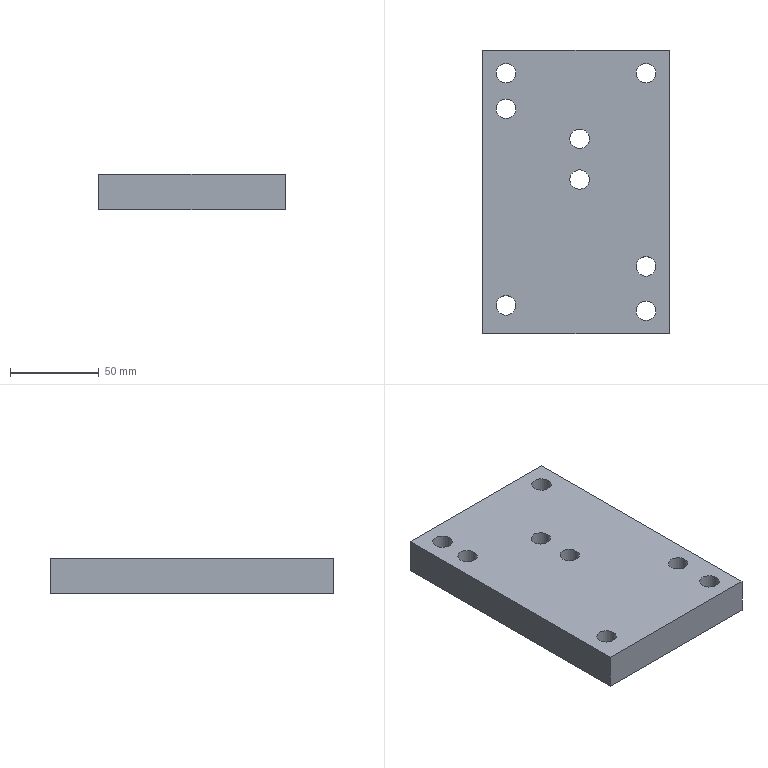Part | STEP file | 108_id3174_x_t | 1 solid | 14 faces | box 105 x 160 x 20 mm | volume 320795 mm3 | cylinder 8 | plane 6 | commonest cylinder face diameters 11 x8
STEP:
#1=CARTESIAN_POINT('',(0.,0.,0.));
#2=DIRECTION('',(0.,0.,1.));
#3=DIRECTION('',(1.,0.,0.));
#4=AXIS2_PLACEMENT_3D('',#1,#2,#3);
#5=CARTESIAN_POINT('',(-309.,100.,105.));
#6=VERTEX_POINT('',#5);
#7=CARTESIAN_POINT('',(-314.5,100.,105.));
#8=DIRECTION('',(0.,0.,1.));
#9=DIRECTION('',(1.,0.,0.));
#10=AXIS2_PLACEMENT_3D('',#7,#8,#9);
#11=CIRCLE('',#10,5.5);
#12=CARTESIAN_POINT('',(-313.5,91.5,105.));
#13=DIRECTION('',(0.,0.,1.));
#14=DIRECTION('',(-1.,0.,0.));
#15=AXIS2_PLACEMENT_3D('',#12,#13,#14);
#16=PLANE('',#15);
#17=CARTESIAN_POINT('',(1.,-8.5));
#18=DIRECTION('',(-1.,0.));
#19=AXIS2_PLACEMENT_2D('',#17,#18);
#20=CIRCLE('',#19,5.5);
#21=(GEOMETRIC_REPRESENTATION_CONTEXT(2)PARAMETRIC_REPRESENTATION_CONTEXT()REPRESENTATION_CONTEXT('',''));
#22=DEFINITIONAL_REPRESENTATION('',(#20),#21);
#23=PCURVE('',#16,#22);
#24=CARTESIAN_POINT('',(-314.5,100.,289.));
#25=DIRECTION('',(0.,0.,-1.));
#26=DIRECTION('',(1.,0.,0.));
#27=AXIS2_PLACEMENT_3D('',#24,#25,#26);
#28=CYLINDRICAL_SURFACE('',#27,5.5);
#29=CARTESIAN_POINT('',(6.283,184.));
#30=DIRECTION('',(-1.,0.));
#31=VECTOR('',#30,1.);
#32=LINE('',#29,#31);
#33=(GEOMETRIC_REPRESENTATION_CONTEXT(2)PARAMETRIC_REPRESENTATION_CONTEXT()REPRESENTATION_CONTEXT('',''));
#34=DEFINITIONAL_REPRESENTATION('',(#32),#33);
#35=PCURVE('',#28,#34);
#36=SURFACE_CURVE('',#11,(#23,#35),.PCURVE_S1.);
#37=EDGE_CURVE('',#6,#6,#36,.T.);
#38=ORIENTED_EDGE('',*,*,#37,.F.);
#39=EDGE_LOOP('',(#38));
#40=FACE_BOUND('',#39,.T.);
#41=CARTESIAN_POINT('',(-271.5,51.,105.));
#42=VERTEX_POINT('',#41);
#43=CARTESIAN_POINT('',(-277.,51.,105.));
#44=DIRECTION('',(0.,0.,-1.));
#45=DIRECTION('',(1.,0.,0.));
#46=AXIS2_PLACEMENT_3D('',#43,#44,#45);
#47=CIRCLE('',#46,5.5);
#48=CARTESIAN_POINT('',(-42.,40.5));
#49=CARTESIAN_POINT('',(-42.,50.026));
#50=CARTESIAN_POINT('',(-33.75,45.263));
#51=CARTESIAN_POINT('',(-25.5,40.5));
#52=CARTESIAN_POINT('',(-33.75,35.737));
#53=CARTESIAN_POINT('',(-42.,30.974));
#54=CARTESIAN_POINT('',(-42.,40.5));
#55=(BOUNDED_CURVE()B_SPLINE_CURVE(2,(#48,#49,#50,#51,#52,#53,#54),.UNSPECIFIED.,.T.,.F.)B_SPLINE_CURVE_WITH_KNOTS((1,2,2,2,2,1),(-2.094,0.,2.094,4.189,6.283,8.378),.UNSPECIFIED.)CURVE()GEOMETRIC_REPRESENTATION_ITEM()RATIONAL_B_SPLINE_CURVE((1.,0.5,1.,0.5,1.,0.5,1.))REPRESENTATION_ITEM(''));
#56=(GEOMETRIC_REPRESENTATION_CONTEXT(2)PARAMETRIC_REPRESENTATION_CONTEXT()REPRESENTATION_CONTEXT('',''));
#57=DEFINITIONAL_REPRESENTATION('',(#55),#56);
#58=PCURVE('',#16,#57);
#59=CARTESIAN_POINT('',(-277.,51.,90.));
#60=DIRECTION('',(0.,0.,1.));
#61=DIRECTION('',(1.,0.,0.));
#62=AXIS2_PLACEMENT_3D('',#59,#60,#61);
#63=CYLINDRICAL_SURFACE('',#62,5.5);
#64=CARTESIAN_POINT('',(6.283,15.));
#65=DIRECTION('',(-1.,0.));
#66=VECTOR('',#65,1.);
#67=LINE('',#64,#66);
#68=(GEOMETRIC_REPRESENTATION_CONTEXT(2)PARAMETRIC_REPRESENTATION_CONTEXT()REPRESENTATION_CONTEXT('',''));
#69=DEFINITIONAL_REPRESENTATION('',(#67),#68);
#70=PCURVE('',#63,#69);
#71=SURFACE_CURVE('',#47,(#58,#70),.PCURVE_S1.);
#72=EDGE_CURVE('',#42,#42,#71,.T.);
#73=ORIENTED_EDGE('',*,*,#72,.T.);
#74=EDGE_LOOP('',(#73));
#75=FACE_BOUND('',#74,.T.);
#76=CARTESIAN_POINT('',(-350.5,29.,105.));
#77=VERTEX_POINT('',#76);
#78=CARTESIAN_POINT('',(-356.,29.,105.));
#79=DIRECTION('',(0.,0.,-1.));
#80=DIRECTION('',(1.,0.,0.));
#81=AXIS2_PLACEMENT_3D('',#78,#79,#80);
#82=CIRCLE('',#81,5.5);
#83=CARTESIAN_POINT('',(37.,62.5));
#84=CARTESIAN_POINT('',(37.,72.026));
#85=CARTESIAN_POINT('',(45.25,67.263));
#86=CARTESIAN_POINT('',(53.5,62.5));
#87=CARTESIAN_POINT('',(45.25,57.737));
#88=CARTESIAN_POINT('',(37.,52.974));
#89=CARTESIAN_POINT('',(37.,62.5));
#90=(BOUNDED_CURVE()B_SPLINE_CURVE(2,(#83,#84,#85,#86,#87,#88,#89),.UNSPECIFIED.,.T.,.F.)B_SPLINE_CURVE_WITH_KNOTS((1,2,2,2,2,1),(-2.094,0.,2.094,4.189,6.283,8.378),.UNSPECIFIED.)CURVE()GEOMETRIC_REPRESENTATION_ITEM()RATIONAL_B_SPLINE_CURVE((1.,0.5,1.,0.5,1.,0.5,1.))REPRESENTATION_ITEM(''));
#91=(GEOMETRIC_REPRESENTATION_CONTEXT(2)PARAMETRIC_REPRESENTATION_CONTEXT()REPRESENTATION_CONTEXT('',''));
#92=DEFINITIONAL_REPRESENTATION('',(#90),#91);
#93=PCURVE('',#16,#92);
#94=CARTESIAN_POINT('',(-356.,29.,90.));
#95=DIRECTION('',(0.,0.,1.));
#96=DIRECTION('',(1.,0.,0.));
#97=AXIS2_PLACEMENT_3D('',#94,#95,#96);
#98=CYLINDRICAL_SURFACE('',#97,5.5);
#99=CARTESIAN_POINT('',(6.283,15.));
#100=DIRECTION('',(-1.,0.));
#101=VECTOR('',#100,1.);
#102=LINE('',#99,#101);
#103=(GEOMETRIC_REPRESENTATION_CONTEXT(2)PARAMETRIC_REPRESENTATION_CONTEXT()REPRESENTATION_CONTEXT('',''));
#104=DEFINITIONAL_REPRESENTATION('',(#102),#103);
#105=PCURVE('',#98,#104);
#106=SURFACE_CURVE('',#82,(#93,#105),.PCURVE_S1.);
#107=EDGE_CURVE('',#77,#77,#106,.T.);
#108=ORIENTED_EDGE('',*,*,#107,.T.);
#109=EDGE_LOOP('',(#108));
#110=FACE_BOUND('',#109,.T.);
#111=CARTESIAN_POINT('',(-271.5,160.,105.));
#112=VERTEX_POINT('',#111);
#113=CARTESIAN_POINT('',(-277.,160.,105.));
#114=DIRECTION('',(0.,0.,-1.));
#115=DIRECTION('',(1.,0.,0.));
#116=AXIS2_PLACEMENT_3D('',#113,#114,#115);
#117=CIRCLE('',#116,5.5);
#118=CARTESIAN_POINT('',(-42.,-68.5));
#119=CARTESIAN_POINT('',(-42.,-58.974));
#120=CARTESIAN_POINT('',(-33.75,-63.737));
#121=CARTESIAN_POINT('',(-25.5,-68.5));
#122=CARTESIAN_POINT('',(-33.75,-73.263));
#123=CARTESIAN_POINT('',(-42.,-78.026));
#124=CARTESIAN_POINT('',(-42.,-68.5));
#125=(BOUNDED_CURVE()B_SPLINE_CURVE(2,(#118,#119,#120,#121,#122,#123,#124),.UNSPECIFIED.,.T.,.F.)B_SPLINE_CURVE_WITH_KNOTS((1,2,2,2,2,1),(-2.094,0.,2.094,4.189,6.283,8.378),.UNSPECIFIED.)CURVE()GEOMETRIC_REPRESENTATION_ITEM()RATIONAL_B_SPLINE_CURVE((1.,0.5,1.,0.5,1.,0.5,1.))REPRESENTATION_ITEM(''));
#126=(GEOMETRIC_REPRESENTATION_CONTEXT(2)PARAMETRIC_REPRESENTATION_CONTEXT()REPRESENTATION_CONTEXT('',''));
#127=DEFINITIONAL_REPRESENTATION('',(#125),#126);
#128=PCURVE('',#16,#127);
#129=CARTESIAN_POINT('',(-277.,160.,90.));
#130=DIRECTION('',(0.,0.,1.));
#131=DIRECTION('',(1.,0.,0.));
#132=AXIS2_PLACEMENT_3D('',#129,#130,#131);
#133=CYLINDRICAL_SURFACE('',#132,5.5);
#134=CARTESIAN_POINT('',(6.283,15.));
#135=DIRECTION('',(-1.,0.));
#136=VECTOR('',#135,1.);
#137=LINE('',#134,#136);
#138=(GEOMETRIC_REPRESENTATION_CONTEXT(2)PARAMETRIC_REPRESENTATION_CONTEXT()REPRESENTATION_CONTEXT('',''));
#139=DEFINITIONAL_REPRESENTATION('',(#137),#138);
#140=PCURVE('',#133,#139);
#141=SURFACE_CURVE('',#117,(#128,#140),.PCURVE_S1.);
#142=EDGE_CURVE('',#112,#112,#141,.T.);
#143=ORIENTED_EDGE('',*,*,#142,.T.);
#144=EDGE_LOOP('',(#143));
#145=FACE_BOUND('',#144,.T.);
#146=CARTESIAN_POINT('',(-369.,173.,105.));
#147=VERTEX_POINT('',#146);
#148=CARTESIAN_POINT('',(-264.,173.,105.));
#149=VERTEX_POINT('',#148);
#150=CARTESIAN_POINT('',(-313.5,173.,105.));
#151=DIRECTION('',(1.,0.,0.));
#152=VECTOR('',#151,1.);
#153=LINE('',#150,#152);
#154=CARTESIAN_POINT('',(0.,-81.5));
#155=DIRECTION('',(-1.,0.));
#156=VECTOR('',#155,1.);
#157=LINE('',#154,#156);
#158=(GEOMETRIC_REPRESENTATION_CONTEXT(2)PARAMETRIC_REPRESENTATION_CONTEXT()REPRESENTATION_CONTEXT('',''));
#159=DEFINITIONAL_REPRESENTATION('',(#157),#158);
#160=PCURVE('',#16,#159);
#161=CARTESIAN_POINT('',(-313.5,173.,90.));
#162=DIRECTION('',(0.,1.,0.));
#163=DIRECTION('',(0.,0.,1.));
#164=AXIS2_PLACEMENT_3D('',#161,#162,#163);
#165=PLANE('',#164);
#166=CARTESIAN_POINT('',(15.,0.));
#167=DIRECTION('',(0.,1.));
#168=VECTOR('',#167,1.);
#169=LINE('',#166,#168);
#170=(GEOMETRIC_REPRESENTATION_CONTEXT(2)PARAMETRIC_REPRESENTATION_CONTEXT()REPRESENTATION_CONTEXT('',''));
#171=DEFINITIONAL_REPRESENTATION('',(#169),#170);
#172=PCURVE('',#165,#171);
#173=SURFACE_CURVE('',#153,(#160,#172),.PCURVE_S1.);
#174=EDGE_CURVE('',#147,#149,#173,.T.);
#175=ORIENTED_EDGE('',*,*,#174,.F.);
#176=CARTESIAN_POINT('',(-369.,13.,105.));
#177=VERTEX_POINT('',#176);
#178=CARTESIAN_POINT('',(-369.,91.5,105.));
#179=DIRECTION('',(0.,1.,0.));
#180=VECTOR('',#179,1.);
#181=LINE('',#178,#180);
#182=CARTESIAN_POINT('',(55.5,0.));
#183=DIRECTION('',(0.,-1.));
#184=VECTOR('',#183,1.);
#185=LINE('',#182,#184);
#186=(GEOMETRIC_REPRESENTATION_CONTEXT(2)PARAMETRIC_REPRESENTATION_CONTEXT()REPRESENTATION_CONTEXT('',''));
#187=DEFINITIONAL_REPRESENTATION('',(#185),#186);
#188=PCURVE('',#16,#187);
#189=CARTESIAN_POINT('',(-369.,91.5,90.));
#190=DIRECTION('',(-1.,0.,0.));
#191=DIRECTION('',(0.,0.,-1.));
#192=AXIS2_PLACEMENT_3D('',#189,#190,#191);
#193=PLANE('',#192);
#194=CARTESIAN_POINT('',(-15.,0.));
#195=DIRECTION('',(0.,-1.));
#196=VECTOR('',#195,1.);
#197=LINE('',#194,#196);
#198=(GEOMETRIC_REPRESENTATION_CONTEXT(2)PARAMETRIC_REPRESENTATION_CONTEXT()REPRESENTATION_CONTEXT('',''));
#199=DEFINITIONAL_REPRESENTATION('',(#197),#198);
#200=PCURVE('',#193,#199);
#201=SURFACE_CURVE('',#181,(#188,#200),.PCURVE_S1.);
#202=EDGE_CURVE('',#177,#147,#201,.T.);
#203=ORIENTED_EDGE('',*,*,#202,.F.);
#204=CARTESIAN_POINT('',(-264.,13.,105.));
#205=VERTEX_POINT('',#204);
#206=CARTESIAN_POINT('',(-313.5,13.,105.));
#207=DIRECTION('',(-1.,0.,0.));
#208=VECTOR('',#207,1.);
#209=LINE('',#206,#208);
#210=CARTESIAN_POINT('',(0.,78.5));
#211=DIRECTION('',(1.,0.));
#212=VECTOR('',#211,1.);
#213=LINE('',#210,#212);
#214=(GEOMETRIC_REPRESENTATION_CONTEXT(2)PARAMETRIC_REPRESENTATION_CONTEXT()REPRESENTATION_CONTEXT('',''));
#215=DEFINITIONAL_REPRESENTATION('',(#213),#214);
#216=PCURVE('',#16,#215);
#217=CARTESIAN_POINT('',(-313.5,13.,90.));
#218=DIRECTION('',(0.,-1.,0.));
#219=DIRECTION('',(0.,0.,-1.));
#220=AXIS2_PLACEMENT_3D('',#217,#218,#219);
#221=PLANE('',#220);
#222=CARTESIAN_POINT('',(-15.,0.));
#223=DIRECTION('',(0.,-1.));
#224=VECTOR('',#223,1.);
#225=LINE('',#222,#224);
#226=(GEOMETRIC_REPRESENTATION_CONTEXT(2)PARAMETRIC_REPRESENTATION_CONTEXT()REPRESENTATION_CONTEXT('',''));
#227=DEFINITIONAL_REPRESENTATION('',(#225),#226);
#228=PCURVE('',#221,#227);
#229=SURFACE_CURVE('',#209,(#216,#228),.PCURVE_S1.);
#230=EDGE_CURVE('',#205,#177,#229,.T.);
#231=ORIENTED_EDGE('',*,*,#230,.F.);
#232=CARTESIAN_POINT('',(-264.,91.5,105.));
#233=DIRECTION('',(0.,-1.,0.));
#234=VECTOR('',#233,1.);
#235=LINE('',#232,#234);
#236=CARTESIAN_POINT('',(-49.5,0.));
#237=DIRECTION('',(0.,1.));
#238=VECTOR('',#237,1.);
#239=LINE('',#236,#238);
#240=(GEOMETRIC_REPRESENTATION_CONTEXT(2)PARAMETRIC_REPRESENTATION_CONTEXT()REPRESENTATION_CONTEXT('',''));
#241=DEFINITIONAL_REPRESENTATION('',(#239),#240);
#242=PCURVE('',#16,#241);
#243=CARTESIAN_POINT('',(-264.,91.5,90.));
#244=DIRECTION('',(1.,0.,0.));
#245=DIRECTION('',(0.,0.,1.));
#246=AXIS2_PLACEMENT_3D('',#243,#244,#245);
#247=PLANE('',#246);
#248=CARTESIAN_POINT('',(15.,0.));
#249=DIRECTION('',(0.,1.));
#250=VECTOR('',#249,1.);
#251=LINE('',#248,#250);
#252=(GEOMETRIC_REPRESENTATION_CONTEXT(2)PARAMETRIC_REPRESENTATION_CONTEXT()REPRESENTATION_CONTEXT('',''));
#253=DEFINITIONAL_REPRESENTATION('',(#251),#252);
#254=PCURVE('',#247,#253);
#255=SURFACE_CURVE('',#235,(#242,#254),.PCURVE_S1.);
#256=EDGE_CURVE('',#149,#205,#255,.T.);
#257=ORIENTED_EDGE('',*,*,#256,.F.);
#258=EDGE_LOOP('',(#175,#203,#231,#257));
#259=FACE_BOUND('',#258,.T.);
#260=CARTESIAN_POINT('',(-350.5,160.,105.));
#261=VERTEX_POINT('',#260);
#262=CARTESIAN_POINT('',(-356.,160.,105.));
#263=DIRECTION('',(0.,0.,-1.));
#264=DIRECTION('',(1.,0.,0.));
#265=AXIS2_PLACEMENT_3D('',#262,#263,#264);
#266=CIRCLE('',#265,5.5);
#267=CARTESIAN_POINT('',(37.,-68.5));
#268=CARTESIAN_POINT('',(37.,-58.974));
#269=CARTESIAN_POINT('',(45.25,-63.737));
#270=CARTESIAN_POINT('',(53.5,-68.5));
#271=CARTESIAN_POINT('',(45.25,-73.263));
#272=CARTESIAN_POINT('',(37.,-78.026));
#273=CARTESIAN_POINT('',(37.,-68.5));
#274=(BOUNDED_CURVE()B_SPLINE_CURVE(2,(#267,#268,#269,#270,#271,#272,#273),.UNSPECIFIED.,.T.,.F.)B_SPLINE_CURVE_WITH_KNOTS((1,2,2,2,2,1),(-2.094,0.,2.094,4.189,6.283,8.378),.UNSPECIFIED.)CURVE()GEOMETRIC_REPRESENTATION_ITEM()RATIONAL_B_SPLINE_CURVE((1.,0.5,1.,0.5,1.,0.5,1.))REPRESENTATION_ITEM(''));
#275=(GEOMETRIC_REPRESENTATION_CONTEXT(2)PARAMETRIC_REPRESENTATION_CONTEXT()REPRESENTATION_CONTEXT('',''));
#276=DEFINITIONAL_REPRESENTATION('',(#274),#275);
#277=PCURVE('',#16,#276);
#278=CARTESIAN_POINT('',(-356.,160.,90.));
#279=DIRECTION('',(0.,0.,1.));
#280=DIRECTION('',(1.,0.,0.));
#281=AXIS2_PLACEMENT_3D('',#278,#279,#280);
#282=CYLINDRICAL_SURFACE('',#281,5.5);
#283=CARTESIAN_POINT('',(6.283,15.));
#284=DIRECTION('',(-1.,0.));
#285=VECTOR('',#284,1.);
#286=LINE('',#283,#285);
#287=(GEOMETRIC_REPRESENTATION_CONTEXT(2)PARAMETRIC_REPRESENTATION_CONTEXT()REPRESENTATION_CONTEXT('',''));
#288=DEFINITIONAL_REPRESENTATION('',(#286),#287);
#289=PCURVE('',#282,#288);
#290=SURFACE_CURVE('',#266,(#277,#289),.PCURVE_S1.);
#291=EDGE_CURVE('',#261,#261,#290,.T.);
#292=ORIENTED_EDGE('',*,*,#291,.T.);
#293=EDGE_LOOP('',(#292));
#294=FACE_BOUND('',#293,.T.);
#295=CARTESIAN_POINT('',(-271.5,26.,105.));
#296=VERTEX_POINT('',#295);
#297=CARTESIAN_POINT('',(-277.,26.,105.));
#298=DIRECTION('',(0.,0.,-1.));
#299=DIRECTION('',(1.,0.,0.));
#300=AXIS2_PLACEMENT_3D('',#297,#298,#299);
#301=CIRCLE('',#300,5.5);
#302=CARTESIAN_POINT('',(-42.,65.5));
#303=CARTESIAN_POINT('',(-42.,75.026));
#304=CARTESIAN_POINT('',(-33.75,70.263));
#305=CARTESIAN_POINT('',(-25.5,65.5));
#306=CARTESIAN_POINT('',(-33.75,60.737));
#307=CARTESIAN_POINT('',(-42.,55.974));
#308=CARTESIAN_POINT('',(-42.,65.5));
#309=(BOUNDED_CURVE()B_SPLINE_CURVE(2,(#302,#303,#304,#305,#306,#307,#308),.UNSPECIFIED.,.T.,.F.)B_SPLINE_CURVE_WITH_KNOTS((1,2,2,2,2,1),(-2.094,0.,2.094,4.189,6.283,8.378),.UNSPECIFIED.)CURVE()GEOMETRIC_REPRESENTATION_ITEM()RATIONAL_B_SPLINE_CURVE((1.,0.5,1.,0.5,1.,0.5,1.))REPRESENTATION_ITEM(''));
#310=(GEOMETRIC_REPRESENTATION_CONTEXT(2)PARAMETRIC_REPRESENTATION_CONTEXT()REPRESENTATION_CONTEXT('',''));
#311=DEFINITIONAL_REPRESENTATION('',(#309),#310);
#312=PCURVE('',#16,#311);
#313=CARTESIAN_POINT('',(-277.,26.,90.));
#314=DIRECTION('',(0.,0.,1.));
#315=DIRECTION('',(1.,0.,0.));
#316=AXIS2_PLACEMENT_3D('',#313,#314,#315);
#317=CYLINDRICAL_SURFACE('',#316,5.5);
#318=CARTESIAN_POINT('',(6.283,15.));
#319=DIRECTION('',(-1.,0.));
#320=VECTOR('',#319,1.);
#321=LINE('',#318,#320);
#322=(GEOMETRIC_REPRESENTATION_CONTEXT(2)PARAMETRIC_REPRESENTATION_CONTEXT()REPRESENTATION_CONTEXT('',''));
#323=DEFINITIONAL_REPRESENTATION('',(#321),#322);
#324=PCURVE('',#317,#323);
#325=SURFACE_CURVE('',#301,(#312,#324),.PCURVE_S1.);
#326=EDGE_CURVE('',#296,#296,#325,.T.);
#327=ORIENTED_EDGE('',*,*,#326,.T.);
#328=EDGE_LOOP('',(#327));
#329=FACE_BOUND('',#328,.T.);
#330=CARTESIAN_POINT('',(-350.5,140.,105.));
#331=VERTEX_POINT('',#330);
#332=CARTESIAN_POINT('',(-356.,140.,105.));
#333=DIRECTION('',(0.,0.,-1.));
#334=DIRECTION('',(1.,0.,0.));
#335=AXIS2_PLACEMENT_3D('',#332,#333,#334);
#336=CIRCLE('',#335,5.5);
#337=CARTESIAN_POINT('',(37.,-48.5));
#338=CARTESIAN_POINT('',(37.,-38.974));
#339=CARTESIAN_POINT('',(45.25,-43.737));
#340=CARTESIAN_POINT('',(53.5,-48.5));
#341=CARTESIAN_POINT('',(45.25,-53.263));
#342=CARTESIAN_POINT('',(37.,-58.026));
#343=CARTESIAN_POINT('',(37.,-48.5));
#344=(BOUNDED_CURVE()B_SPLINE_CURVE(2,(#337,#338,#339,#340,#341,#342,#343),.UNSPECIFIED.,.T.,.F.)B_SPLINE_CURVE_WITH_KNOTS((1,2,2,2,2,1),(-2.094,0.,2.094,4.189,6.283,8.378),.UNSPECIFIED.)CURVE()GEOMETRIC_REPRESENTATION_ITEM()RATIONAL_B_SPLINE_CURVE((1.,0.5,1.,0.5,1.,0.5,1.))REPRESENTATION_ITEM(''));
#345=(GEOMETRIC_REPRESENTATION_CONTEXT(2)PARAMETRIC_REPRESENTATION_CONTEXT()REPRESENTATION_CONTEXT('',''));
#346=DEFINITIONAL_REPRESENTATION('',(#344),#345);
#347=PCURVE('',#16,#346);
#348=CARTESIAN_POINT('',(-356.,140.,90.));
#349=DIRECTION('',(0.,0.,1.));
#350=DIRECTION('',(1.,0.,0.));
#351=AXIS2_PLACEMENT_3D('',#348,#349,#350);
#352=CYLINDRICAL_SURFACE('',#351,5.5);
#353=CARTESIAN_POINT('',(6.283,15.));
#354=DIRECTION('',(-1.,0.));
#355=VECTOR('',#354,1.);
#356=LINE('',#353,#355);
#357=(GEOMETRIC_REPRESENTATION_CONTEXT(2)PARAMETRIC_REPRESENTATION_CONTEXT()REPRESENTATION_CONTEXT('',''));
#358=DEFINITIONAL_REPRESENTATION('',(#356),#357);
#359=PCURVE('',#352,#358);
#360=SURFACE_CURVE('',#336,(#347,#359),.PCURVE_S1.);
#361=EDGE_CURVE('',#331,#331,#360,.T.);
#362=ORIENTED_EDGE('',*,*,#361,.T.);
#363=EDGE_LOOP('',(#362));
#364=FACE_BOUND('',#363,.T.);
#365=CARTESIAN_POINT('',(-309.,123.,105.));
#366=VERTEX_POINT('',#365);
#367=CARTESIAN_POINT('',(-314.5,123.,105.));
#368=DIRECTION('',(0.,0.,-1.));
#369=DIRECTION('',(1.,0.,0.));
#370=AXIS2_PLACEMENT_3D('',#367,#368,#369);
#371=CIRCLE('',#370,5.5);
#372=CARTESIAN_POINT('',(-4.5,-31.5));
#373=CARTESIAN_POINT('',(-4.5,-21.974));
#374=CARTESIAN_POINT('',(3.75,-26.737));
#375=CARTESIAN_POINT('',(12.,-31.5));
#376=CARTESIAN_POINT('',(3.75,-36.263));
#377=CARTESIAN_POINT('',(-4.5,-41.026));
#378=CARTESIAN_POINT('',(-4.5,-31.5));
#379=(BOUNDED_CURVE()B_SPLINE_CURVE(2,(#372,#373,#374,#375,#376,#377,#378),.UNSPECIFIED.,.T.,.F.)B_SPLINE_CURVE_WITH_KNOTS((1,2,2,2,2,1),(-2.094,0.,2.094,4.189,6.283,8.378),.UNSPECIFIED.)CURVE()GEOMETRIC_REPRESENTATION_ITEM()RATIONAL_B_SPLINE_CURVE((1.,0.5,1.,0.5,1.,0.5,1.))REPRESENTATION_ITEM(''));
#380=(GEOMETRIC_REPRESENTATION_CONTEXT(2)PARAMETRIC_REPRESENTATION_CONTEXT()REPRESENTATION_CONTEXT('',''));
#381=DEFINITIONAL_REPRESENTATION('',(#379),#380);
#382=PCURVE('',#16,#381);
#383=CARTESIAN_POINT('',(-314.5,123.,289.));
#384=DIRECTION('',(0.,0.,-1.));
#385=DIRECTION('',(1.,0.,0.));
#386=AXIS2_PLACEMENT_3D('',#383,#384,#385);
#387=CYLINDRICAL_SURFACE('',#386,5.5);
#388=CARTESIAN_POINT('',(0.,184.));
#389=DIRECTION('',(1.,0.));
#390=VECTOR('',#389,1.);
#391=LINE('',#388,#390);
#392=(GEOMETRIC_REPRESENTATION_CONTEXT(2)PARAMETRIC_REPRESENTATION_CONTEXT()REPRESENTATION_CONTEXT('',''));
#393=DEFINITIONAL_REPRESENTATION('',(#391),#392);
#394=PCURVE('',#387,#393);
#395=SURFACE_CURVE('',#371,(#382,#394),.PCURVE_S1.);
#396=EDGE_CURVE('',#366,#366,#395,.T.);
#397=ORIENTED_EDGE('',*,*,#396,.T.);
#398=EDGE_LOOP('',(#397));
#399=FACE_BOUND('',#398,.T.);
#400=ADVANCED_FACE('',(#40,#75,#110,#145,#259,#294,#329,#364,#399),#16,.T.);
#401=CARTESIAN_POINT('',(-320.,100.,85.));
#402=VERTEX_POINT('',#401);
#403=CARTESIAN_POINT('',(-309.,100.,85.));
#404=VERTEX_POINT('',#403);
#405=CARTESIAN_POINT('',(-314.5,100.,85.));
#406=DIRECTION('',(0.,0.,-1.));
#407=DIRECTION('',(-1.,0.,0.));
#408=AXIS2_PLACEMENT_3D('',#405,#406,#407);
#409=CIRCLE('',#408,5.5);
#410=CARTESIAN_POINT('',(-313.5,91.5,85.));
#411=DIRECTION('',(0.,0.,-1.));
#412=DIRECTION('',(1.,0.,0.));
#413=AXIS2_PLACEMENT_3D('',#410,#411,#412);
#414=PLANE('',#413);
#415=CARTESIAN_POINT('',(-1.,-8.5));
#416=DIRECTION('',(-1.,0.));
#417=AXIS2_PLACEMENT_2D('',#415,#416);
#418=CIRCLE('',#417,5.5);
#419=(GEOMETRIC_REPRESENTATION_CONTEXT(2)PARAMETRIC_REPRESENTATION_CONTEXT()REPRESENTATION_CONTEXT('',''));
#420=DEFINITIONAL_REPRESENTATION('',(#418),#419);
#421=PCURVE('',#414,#420);
#422=CARTESIAN_POINT('',(3.142,204.));
#423=DIRECTION('',(1.,0.));
#424=VECTOR('',#423,1.);
#425=LINE('',#422,#424);
#426=(GEOMETRIC_REPRESENTATION_CONTEXT(2)PARAMETRIC_REPRESENTATION_CONTEXT()REPRESENTATION_CONTEXT('',''));
#427=DEFINITIONAL_REPRESENTATION('',(#425),#426);
#428=PCURVE('',#28,#427);
#429=SURFACE_CURVE('',#409,(#421,#428),.PCURVE_S1.);
#430=EDGE_CURVE('',#402,#404,#429,.T.);
#431=ORIENTED_EDGE('',*,*,#430,.F.);
#432=CARTESIAN_POINT('',(-314.5,100.,85.));
#433=DIRECTION('',(0.,0.,-1.));
#434=DIRECTION('',(-1.,0.,0.));
#435=AXIS2_PLACEMENT_3D('',#432,#433,#434);
#436=CIRCLE('',#435,5.5);
#437=CARTESIAN_POINT('',(-1.,-8.5));
#438=DIRECTION('',(-1.,0.));
#439=AXIS2_PLACEMENT_2D('',#437,#438);
#440=CIRCLE('',#439,5.5);
#441=(GEOMETRIC_REPRESENTATION_CONTEXT(2)PARAMETRIC_REPRESENTATION_CONTEXT()REPRESENTATION_CONTEXT('',''));
#442=DEFINITIONAL_REPRESENTATION('',(#440),#441);
#443=PCURVE('',#414,#442);
#444=CARTESIAN_POINT('',(-3.142,204.));
#445=DIRECTION('',(1.,0.));
#446=VECTOR('',#445,1.);
#447=LINE('',#444,#446);
#448=(GEOMETRIC_REPRESENTATION_CONTEXT(2)PARAMETRIC_REPRESENTATION_CONTEXT()REPRESENTATION_CONTEXT('',''));
#449=DEFINITIONAL_REPRESENTATION('',(#447),#448);
#450=PCURVE('',#28,#449);
#451=SURFACE_CURVE('',#436,(#443,#450),.PCURVE_S1.);
#452=EDGE_CURVE('',#404,#402,#451,.T.);
#453=ORIENTED_EDGE('',*,*,#452,.F.);
#454=EDGE_LOOP('',(#431,#453));
#455=FACE_BOUND('',#454,.T.);
#456=CARTESIAN_POINT('',(-282.5,51.,85.));
#457=VERTEX_POINT('',#456);
#458=CARTESIAN_POINT('',(-271.5,51.,85.));
#459=VERTEX_POINT('',#458);
#460=CARTESIAN_POINT('',(-277.,51.,85.));
#461=DIRECTION('',(0.,0.,1.));
#462=DIRECTION('',(-1.,0.,0.));
#463=AXIS2_PLACEMENT_3D('',#460,#461,#462);
#464=CIRCLE('',#463,5.5);
#465=CARTESIAN_POINT('',(31.,40.5));
#466=CARTESIAN_POINT('',(31.,50.026));
#467=CARTESIAN_POINT('',(39.25,45.263));
#468=CARTESIAN_POINT('',(47.5,40.5));
#469=CARTESIAN_POINT('',(39.25,35.737));
#470=CARTESIAN_POINT('',(31.,30.974));
#471=CARTESIAN_POINT('',(31.,40.5));
#472=(BOUNDED_CURVE()B_SPLINE_CURVE(2,(#465,#466,#467,#468,#469,#470,#471),.UNSPECIFIED.,.T.,.F.)B_SPLINE_CURVE_WITH_KNOTS((1,2,2,2,2,1),(-2.094,0.,2.094,4.189,6.283,8.378),.UNSPECIFIED.)CURVE()GEOMETRIC_REPRESENTATION_ITEM()RATIONAL_B_SPLINE_CURVE((1.,0.5,1.,0.5,1.,0.5,1.))REPRESENTATION_ITEM(''));
#473=(GEOMETRIC_REPRESENTATION_CONTEXT(2)PARAMETRIC_REPRESENTATION_CONTEXT()REPRESENTATION_CONTEXT('',''));
#474=DEFINITIONAL_REPRESENTATION('',(#472),#473);
#475=PCURVE('',#414,#474);
#476=CARTESIAN_POINT('',(3.142,-5.));
#477=DIRECTION('',(1.,0.));
#478=VECTOR('',#477,1.);
#479=LINE('',#476,#478);
#480=(GEOMETRIC_REPRESENTATION_CONTEXT(2)PARAMETRIC_REPRESENTATION_CONTEXT()REPRESENTATION_CONTEXT('',''));
#481=DEFINITIONAL_REPRESENTATION('',(#479),#480);
#482=PCURVE('',#63,#481);
#483=SURFACE_CURVE('',#464,(#475,#482),.PCURVE_S1.);
#484=EDGE_CURVE('',#457,#459,#483,.T.);
#485=ORIENTED_EDGE('',*,*,#484,.T.);
#486=CARTESIAN_POINT('',(-277.,51.,85.));
#487=DIRECTION('',(0.,0.,1.));
#488=DIRECTION('',(-1.,0.,0.));
#489=AXIS2_PLACEMENT_3D('',#486,#487,#488);
#490=CIRCLE('',#489,5.5);
#491=CARTESIAN_POINT('',(31.,40.5));
#492=CARTESIAN_POINT('',(31.,50.026));
#493=CARTESIAN_POINT('',(39.25,45.263));
#494=CARTESIAN_POINT('',(47.5,40.5));
#495=CARTESIAN_POINT('',(39.25,35.737));
#496=CARTESIAN_POINT('',(31.,30.974));
#497=CARTESIAN_POINT('',(31.,40.5));
#498=(BOUNDED_CURVE()B_SPLINE_CURVE(2,(#491,#492,#493,#494,#495,#496,#497),.UNSPECIFIED.,.T.,.F.)B_SPLINE_CURVE_WITH_KNOTS((1,2,2,2,2,1),(-2.094,0.,2.094,4.189,6.283,8.378),.UNSPECIFIED.)CURVE()GEOMETRIC_REPRESENTATION_ITEM()RATIONAL_B_SPLINE_CURVE((1.,0.5,1.,0.5,1.,0.5,1.))REPRESENTATION_ITEM(''));
#499=(GEOMETRIC_REPRESENTATION_CONTEXT(2)PARAMETRIC_REPRESENTATION_CONTEXT()REPRESENTATION_CONTEXT('',''));
#500=DEFINITIONAL_REPRESENTATION('',(#498),#499);
#501=PCURVE('',#414,#500);
#502=CARTESIAN_POINT('',(-3.142,-5.));
#503=DIRECTION('',(1.,0.));
#504=VECTOR('',#503,1.);
#505=LINE('',#502,#504);
#506=(GEOMETRIC_REPRESENTATION_CONTEXT(2)PARAMETRIC_REPRESENTATION_CONTEXT()REPRESENTATION_CONTEXT('',''));
#507=DEFINITIONAL_REPRESENTATION('',(#505),#506);
#508=PCURVE('',#63,#507);
#509=SURFACE_CURVE('',#490,(#501,#508),.PCURVE_S1.);
#510=EDGE_CURVE('',#459,#457,#509,.T.);
#511=ORIENTED_EDGE('',*,*,#510,.T.);
#512=EDGE_LOOP('',(#485,#511));
#513=FACE_BOUND('',#512,.T.);
#514=CARTESIAN_POINT('',(-361.5,29.,85.));
#515=VERTEX_POINT('',#514);
#516=CARTESIAN_POINT('',(-350.5,29.,85.));
#517=VERTEX_POINT('',#516);
#518=CARTESIAN_POINT('',(-356.,29.,85.));
#519=DIRECTION('',(0.,0.,1.));
#520=DIRECTION('',(-1.,0.,0.));
#521=AXIS2_PLACEMENT_3D('',#518,#519,#520);
#522=CIRCLE('',#521,5.5);
#523=CARTESIAN_POINT('',(-48.,62.5));
#524=CARTESIAN_POINT('',(-48.,72.026));
#525=CARTESIAN_POINT('',(-39.75,67.263));
#526=CARTESIAN_POINT('',(-31.5,62.5));
#527=CARTESIAN_POINT('',(-39.75,57.737));
#528=CARTESIAN_POINT('',(-48.,52.974));
#529=CARTESIAN_POINT('',(-48.,62.5));
#530=(BOUNDED_CURVE()B_SPLINE_CURVE(2,(#523,#524,#525,#526,#527,#528,#529),.UNSPECIFIED.,.T.,.F.)B_SPLINE_CURVE_WITH_KNOTS((1,2,2,2,2,1),(-2.094,0.,2.094,4.189,6.283,8.378),.UNSPECIFIED.)CURVE()GEOMETRIC_REPRESENTATION_ITEM()RATIONAL_B_SPLINE_CURVE((1.,0.5,1.,0.5,1.,0.5,1.))REPRESENTATION_ITEM(''));
#531=(GEOMETRIC_REPRESENTATION_CONTEXT(2)PARAMETRIC_REPRESENTATION_CONTEXT()REPRESENTATION_CONTEXT('',''));
#532=DEFINITIONAL_REPRESENTATION('',(#530),#531);
#533=PCURVE('',#414,#532);
#534=CARTESIAN_POINT('',(3.142,-5.));
#535=DIRECTION('',(1.,0.));
#536=VECTOR('',#535,1.);
#537=LINE('',#534,#536);
#538=(GEOMETRIC_REPRESENTATION_CONTEXT(2)PARAMETRIC_REPRESENTATION_CONTEXT()REPRESENTATION_CONTEXT('',''));
#539=DEFINITIONAL_REPRESENTATION('',(#537),#538);
#540=PCURVE('',#98,#539);
#541=SURFACE_CURVE('',#522,(#533,#540),.PCURVE_S1.);
#542=EDGE_CURVE('',#515,#517,#541,.T.);
#543=ORIENTED_EDGE('',*,*,#542,.T.);
#544=CARTESIAN_POINT('',(-356.,29.,85.));
#545=DIRECTION('',(0.,0.,1.));
#546=DIRECTION('',(-1.,0.,0.));
#547=AXIS2_PLACEMENT_3D('',#544,#545,#546);
#548=CIRCLE('',#547,5.5);
#549=CARTESIAN_POINT('',(-48.,62.5));
#550=CARTESIAN_POINT('',(-48.,72.026));
#551=CARTESIAN_POINT('',(-39.75,67.263));
#552=CARTESIAN_POINT('',(-31.5,62.5));
#553=CARTESIAN_POINT('',(-39.75,57.737));
#554=CARTESIAN_POINT('',(-48.,52.974));
#555=CARTESIAN_POINT('',(-48.,62.5));
#556=(BOUNDED_CURVE()B_SPLINE_CURVE(2,(#549,#550,#551,#552,#553,#554,#555),.UNSPECIFIED.,.T.,.F.)B_SPLINE_CURVE_WITH_KNOTS((1,2,2,2,2,1),(-2.094,0.,2.094,4.189,6.283,8.378),.UNSPECIFIED.)CURVE()GEOMETRIC_REPRESENTATION_ITEM()RATIONAL_B_SPLINE_CURVE((1.,0.5,1.,0.5,1.,0.5,1.))REPRESENTATION_ITEM(''));
#557=(GEOMETRIC_REPRESENTATION_CONTEXT(2)PARAMETRIC_REPRESENTATION_CONTEXT()REPRESENTATION_CONTEXT('',''));
#558=DEFINITIONAL_REPRESENTATION('',(#556),#557);
#559=PCURVE('',#414,#558);
#560=CARTESIAN_POINT('',(-3.142,-5.));
#561=DIRECTION('',(1.,0.));
#562=VECTOR('',#561,1.);
#563=LINE('',#560,#562);
#564=(GEOMETRIC_REPRESENTATION_CONTEXT(2)PARAMETRIC_REPRESENTATION_CONTEXT()REPRESENTATION_CONTEXT('',''));
#565=DEFINITIONAL_REPRESENTATION('',(#563),#564);
#566=PCURVE('',#98,#565);
#567=SURFACE_CURVE('',#548,(#559,#566),.PCURVE_S1.);
#568=EDGE_CURVE('',#517,#515,#567,.T.);
#569=ORIENTED_EDGE('',*,*,#568,.T.);
#570=EDGE_LOOP('',(#543,#569));
#571=FACE_BOUND('',#570,.T.);
#572=CARTESIAN_POINT('',(-282.5,160.,85.));
#573=VERTEX_POINT('',#572);
#574=CARTESIAN_POINT('',(-271.5,160.,85.));
#575=VERTEX_POINT('',#574);
#576=CARTESIAN_POINT('',(-277.,160.,85.));
#577=DIRECTION('',(0.,0.,1.));
#578=DIRECTION('',(-1.,0.,0.));
#579=AXIS2_PLACEMENT_3D('',#576,#577,#578);
#580=CIRCLE('',#579,5.5);
#581=CARTESIAN_POINT('',(31.,-68.5));
#582=CARTESIAN_POINT('',(31.,-58.974));
#583=CARTESIAN_POINT('',(39.25,-63.737));
#584=CARTESIAN_POINT('',(47.5,-68.5));
#585=CARTESIAN_POINT('',(39.25,-73.263));
#586=CARTESIAN_POINT('',(31.,-78.026));
#587=CARTESIAN_POINT('',(31.,-68.5));
#588=(BOUNDED_CURVE()B_SPLINE_CURVE(2,(#581,#582,#583,#584,#585,#586,#587),.UNSPECIFIED.,.T.,.F.)B_SPLINE_CURVE_WITH_KNOTS((1,2,2,2,2,1),(-2.094,0.,2.094,4.189,6.283,8.378),.UNSPECIFIED.)CURVE()GEOMETRIC_REPRESENTATION_ITEM()RATIONAL_B_SPLINE_CURVE((1.,0.5,1.,0.5,1.,0.5,1.))REPRESENTATION_ITEM(''));
#589=(GEOMETRIC_REPRESENTATION_CONTEXT(2)PARAMETRIC_REPRESENTATION_CONTEXT()REPRESENTATION_CONTEXT('',''));
#590=DEFINITIONAL_REPRESENTATION('',(#588),#589);
#591=PCURVE('',#414,#590);
#592=CARTESIAN_POINT('',(3.142,-5.));
#593=DIRECTION('',(1.,0.));
#594=VECTOR('',#593,1.);
#595=LINE('',#592,#594);
#596=(GEOMETRIC_REPRESENTATION_CONTEXT(2)PARAMETRIC_REPRESENTATION_CONTEXT()REPRESENTATION_CONTEXT('',''));
#597=DEFINITIONAL_REPRESENTATION('',(#595),#596);
#598=PCURVE('',#133,#597);
#599=SURFACE_CURVE('',#580,(#591,#598),.PCURVE_S1.);
#600=EDGE_CURVE('',#573,#575,#599,.T.);
#601=ORIENTED_EDGE('',*,*,#600,.T.);
#602=CARTESIAN_POINT('',(-277.,160.,85.));
#603=DIRECTION('',(0.,0.,1.));
#604=DIRECTION('',(-1.,0.,0.));
#605=AXIS2_PLACEMENT_3D('',#602,#603,#604);
#606=CIRCLE('',#605,5.5);
#607=CARTESIAN_POINT('',(31.,-68.5));
#608=CARTESIAN_POINT('',(31.,-58.974));
#609=CARTESIAN_POINT('',(39.25,-63.737));
#610=CARTESIAN_POINT('',(47.5,-68.5));
#611=CARTESIAN_POINT('',(39.25,-73.263));
#612=CARTESIAN_POINT('',(31.,-78.026));
#613=CARTESIAN_POINT('',(31.,-68.5));
#614=(BOUNDED_CURVE()B_SPLINE_CURVE(2,(#607,#608,#609,#610,#611,#612,#613),.UNSPECIFIED.,.T.,.F.)B_SPLINE_CURVE_WITH_KNOTS((1,2,2,2,2,1),(-2.094,0.,2.094,4.189,6.283,8.378),.UNSPECIFIED.)CURVE()GEOMETRIC_REPRESENTATION_ITEM()RATIONAL_B_SPLINE_CURVE((1.,0.5,1.,0.5,1.,0.5,1.))REPRESENTATION_ITEM(''));
#615=(GEOMETRIC_REPRESENTATION_CONTEXT(2)PARAMETRIC_REPRESENTATION_CONTEXT()REPRESENTATION_CONTEXT('',''));
#616=DEFINITIONAL_REPRESENTATION('',(#614),#615);
#617=PCURVE('',#414,#616);
#618=CARTESIAN_POINT('',(-3.142,-5.));
#619=DIRECTION('',(1.,0.));
#620=VECTOR('',#619,1.);
#621=LINE('',#618,#620);
#622=(GEOMETRIC_REPRESENTATION_CONTEXT(2)PARAMETRIC_REPRESENTATION_CONTEXT()REPRESENTATION_CONTEXT('',''));
#623=DEFINITIONAL_REPRESENTATION('',(#621),#622);
#624=PCURVE('',#133,#623);
#625=SURFACE_CURVE('',#606,(#617,#624),.PCURVE_S1.);
#626=EDGE_CURVE('',#575,#573,#625,.T.);
#627=ORIENTED_EDGE('',*,*,#626,.T.);
#628=EDGE_LOOP('',(#601,#627));
#629=FACE_BOUND('',#628,.T.);
#630=CARTESIAN_POINT('',(-264.,13.,85.));
#631=VERTEX_POINT('',#630);
#632=CARTESIAN_POINT('',(-264.,173.,85.));
#633=VERTEX_POINT('',#632);
#634=CARTESIAN_POINT('',(-264.,91.5,85.));
#635=DIRECTION('',(0.,1.,0.));
#636=VECTOR('',#635,1.);
#637=LINE('',#634,#636);
#638=CARTESIAN_POINT('',(49.5,0.));
#639=DIRECTION('',(0.,-1.));
#640=VECTOR('',#639,1.);
#641=LINE('',#638,#640);
#642=(GEOMETRIC_REPRESENTATION_CONTEXT(2)PARAMETRIC_REPRESENTATION_CONTEXT()REPRESENTATION_CONTEXT('',''));
#643=DEFINITIONAL_REPRESENTATION('',(#641),#642);
#644=PCURVE('',#414,#643);
#645=CARTESIAN_POINT('',(-5.,0.));
#646=DIRECTION('',(0.,-1.));
#647=VECTOR('',#646,1.);
#648=LINE('',#645,#647);
#649=(GEOMETRIC_REPRESENTATION_CONTEXT(2)PARAMETRIC_REPRESENTATION_CONTEXT()REPRESENTATION_CONTEXT('',''));
#650=DEFINITIONAL_REPRESENTATION('',(#648),#649);
#651=PCURVE('',#247,#650);
#652=SURFACE_CURVE('',#637,(#644,#651),.PCURVE_S1.);
#653=EDGE_CURVE('',#631,#633,#652,.T.);
#654=ORIENTED_EDGE('',*,*,#653,.F.);
#655=CARTESIAN_POINT('',(-369.,13.,85.));
#656=VERTEX_POINT('',#655);
#657=CARTESIAN_POINT('',(-313.5,13.,85.));
#658=DIRECTION('',(1.,0.,0.));
#659=VECTOR('',#658,1.);
#660=LINE('',#657,#659);
#661=CARTESIAN_POINT('',(0.,78.5));
#662=DIRECTION('',(1.,0.));
#663=VECTOR('',#662,1.);
#664=LINE('',#661,#663);
#665=(GEOMETRIC_REPRESENTATION_CONTEXT(2)PARAMETRIC_REPRESENTATION_CONTEXT()REPRESENTATION_CONTEXT('',''));
#666=DEFINITIONAL_REPRESENTATION('',(#664),#665);
#667=PCURVE('',#414,#666);
#668=CARTESIAN_POINT('',(5.,0.));
#669=DIRECTION('',(0.,1.));
#670=VECTOR('',#669,1.);
#671=LINE('',#668,#670);
#672=(GEOMETRIC_REPRESENTATION_CONTEXT(2)PARAMETRIC_REPRESENTATION_CONTEXT()REPRESENTATION_CONTEXT('',''));
#673=DEFINITIONAL_REPRESENTATION('',(#671),#672);
#674=PCURVE('',#221,#673);
#675=SURFACE_CURVE('',#660,(#667,#674),.PCURVE_S1.);
#676=EDGE_CURVE('',#656,#631,#675,.T.);
#677=ORIENTED_EDGE('',*,*,#676,.F.);
#678=CARTESIAN_POINT('',(-369.,173.,85.));
#679=VERTEX_POINT('',#678);
#680=CARTESIAN_POINT('',(-369.,91.5,85.));
#681=DIRECTION('',(0.,-1.,0.));
#682=VECTOR('',#681,1.);
#683=LINE('',#680,#682);
#684=CARTESIAN_POINT('',(-55.5,0.));
#685=DIRECTION('',(0.,1.));
#686=VECTOR('',#685,1.);
#687=LINE('',#684,#686);
#688=(GEOMETRIC_REPRESENTATION_CONTEXT(2)PARAMETRIC_REPRESENTATION_CONTEXT()REPRESENTATION_CONTEXT('',''));
#689=DEFINITIONAL_REPRESENTATION('',(#687),#688);
#690=PCURVE('',#414,#689);
#691=CARTESIAN_POINT('',(5.,0.));
#692=DIRECTION('',(0.,1.));
#693=VECTOR('',#692,1.);
#694=LINE('',#691,#693);
#695=(GEOMETRIC_REPRESENTATION_CONTEXT(2)PARAMETRIC_REPRESENTATION_CONTEXT()REPRESENTATION_CONTEXT('',''));
#696=DEFINITIONAL_REPRESENTATION('',(#694),#695);
#697=PCURVE('',#193,#696);
#698=SURFACE_CURVE('',#683,(#690,#697),.PCURVE_S1.);
#699=EDGE_CURVE('',#679,#656,#698,.T.);
#700=ORIENTED_EDGE('',*,*,#699,.F.);
#701=CARTESIAN_POINT('',(-313.5,173.,85.));
#702=DIRECTION('',(-1.,0.,0.));
#703=VECTOR('',#702,1.);
#704=LINE('',#701,#703);
#705=CARTESIAN_POINT('',(0.,-81.5));
#706=DIRECTION('',(-1.,0.));
#707=VECTOR('',#706,1.);
#708=LINE('',#705,#707);
#709=(GEOMETRIC_REPRESENTATION_CONTEXT(2)PARAMETRIC_REPRESENTATION_CONTEXT()REPRESENTATION_CONTEXT('',''));
#710=DEFINITIONAL_REPRESENTATION('',(#708),#709);
#711=PCURVE('',#414,#710);
#712=CARTESIAN_POINT('',(-5.,0.));
#713=DIRECTION('',(0.,-1.));
#714=VECTOR('',#713,1.);
#715=LINE('',#712,#714);
#716=(GEOMETRIC_REPRESENTATION_CONTEXT(2)PARAMETRIC_REPRESENTATION_CONTEXT()REPRESENTATION_CONTEXT('',''));
#717=DEFINITIONAL_REPRESENTATION('',(#715),#716);
#718=PCURVE('',#165,#717);
#719=SURFACE_CURVE('',#704,(#711,#718),.PCURVE_S1.);
#720=EDGE_CURVE('',#633,#679,#719,.T.);
#721=ORIENTED_EDGE('',*,*,#720,.F.);
#722=EDGE_LOOP('',(#654,#677,#700,#721));
#723=FACE_BOUND('',#722,.T.);
#724=CARTESIAN_POINT('',(-361.5,160.,85.));
#725=VERTEX_POINT('',#724);
#726=CARTESIAN_POINT('',(-350.5,160.,85.));
#727=VERTEX_POINT('',#726);
#728=CARTESIAN_POINT('',(-356.,160.,85.));
#729=DIRECTION('',(0.,0.,1.));
#730=DIRECTION('',(-1.,0.,0.));
#731=AXIS2_PLACEMENT_3D('',#728,#729,#730);
#732=CIRCLE('',#731,5.5);
#733=CARTESIAN_POINT('',(-48.,-68.5));
#734=CARTESIAN_POINT('',(-48.,-58.974));
#735=CARTESIAN_POINT('',(-39.75,-63.737));
#736=CARTESIAN_POINT('',(-31.5,-68.5));
#737=CARTESIAN_POINT('',(-39.75,-73.263));
#738=CARTESIAN_POINT('',(-48.,-78.026));
#739=CARTESIAN_POINT('',(-48.,-68.5));
#740=(BOUNDED_CURVE()B_SPLINE_CURVE(2,(#733,#734,#735,#736,#737,#738,#739),.UNSPECIFIED.,.T.,.F.)B_SPLINE_CURVE_WITH_KNOTS((1,2,2,2,2,1),(-2.094,0.,2.094,4.189,6.283,8.378),.UNSPECIFIED.)CURVE()GEOMETRIC_REPRESENTATION_ITEM()RATIONAL_B_SPLINE_CURVE((1.,0.5,1.,0.5,1.,0.5,1.))REPRESENTATION_ITEM(''));
#741=(GEOMETRIC_REPRESENTATION_CONTEXT(2)PARAMETRIC_REPRESENTATION_CONTEXT()REPRESENTATION_CONTEXT('',''));
#742=DEFINITIONAL_REPRESENTATION('',(#740),#741);
#743=PCURVE('',#414,#742);
#744=CARTESIAN_POINT('',(3.142,-5.));
#745=DIRECTION('',(1.,0.));
#746=VECTOR('',#745,1.);
#747=LINE('',#744,#746);
#748=(GEOMETRIC_REPRESENTATION_CONTEXT(2)PARAMETRIC_REPRESENTATION_CONTEXT()REPRESENTATION_CONTEXT('',''));
#749=DEFINITIONAL_REPRESENTATION('',(#747),#748);
#750=PCURVE('',#282,#749);
#751=SURFACE_CURVE('',#732,(#743,#750),.PCURVE_S1.);
#752=EDGE_CURVE('',#725,#727,#751,.T.);
#753=ORIENTED_EDGE('',*,*,#752,.T.);
#754=CARTESIAN_POINT('',(-356.,160.,85.));
#755=DIRECTION('',(0.,0.,1.));
#756=DIRECTION('',(-1.,0.,0.));
#757=AXIS2_PLACEMENT_3D('',#754,#755,#756);
#758=CIRCLE('',#757,5.5);
#759=CARTESIAN_POINT('',(-48.,-68.5));
#760=CARTESIAN_POINT('',(-48.,-58.974));
#761=CARTESIAN_POINT('',(-39.75,-63.737));
#762=CARTESIAN_POINT('',(-31.5,-68.5));
#763=CARTESIAN_POINT('',(-39.75,-73.263));
#764=CARTESIAN_POINT('',(-48.,-78.026));
#765=CARTESIAN_POINT('',(-48.,-68.5));
#766=(BOUNDED_CURVE()B_SPLINE_CURVE(2,(#759,#760,#761,#762,#763,#764,#765),.UNSPECIFIED.,.T.,.F.)B_SPLINE_CURVE_WITH_KNOTS((1,2,2,2,2,1),(-2.094,0.,2.094,4.189,6.283,8.378),.UNSPECIFIED.)CURVE()GEOMETRIC_REPRESENTATION_ITEM()RATIONAL_B_SPLINE_CURVE((1.,0.5,1.,0.5,1.,0.5,1.))REPRESENTATION_ITEM(''));
#767=(GEOMETRIC_REPRESENTATION_CONTEXT(2)PARAMETRIC_REPRESENTATION_CONTEXT()REPRESENTATION_CONTEXT('',''));
#768=DEFINITIONAL_REPRESENTATION('',(#766),#767);
#769=PCURVE('',#414,#768);
#770=CARTESIAN_POINT('',(-3.142,-5.));
#771=DIRECTION('',(1.,0.));
#772=VECTOR('',#771,1.);
#773=LINE('',#770,#772);
#774=(GEOMETRIC_REPRESENTATION_CONTEXT(2)PARAMETRIC_REPRESENTATION_CONTEXT()REPRESENTATION_CONTEXT('',''));
#775=DEFINITIONAL_REPRESENTATION('',(#773),#774);
#776=PCURVE('',#282,#775);
#777=SURFACE_CURVE('',#758,(#769,#776),.PCURVE_S1.);
#778=EDGE_CURVE('',#727,#725,#777,.T.);
#779=ORIENTED_EDGE('',*,*,#778,.T.);
#780=EDGE_LOOP('',(#753,#779));
#781=FACE_BOUND('',#780,.T.);
#782=CARTESIAN_POINT('',(-282.5,26.,85.));
#783=VERTEX_POINT('',#782);
#784=CARTESIAN_POINT('',(-271.5,26.,85.));
#785=VERTEX_POINT('',#784);
#786=CARTESIAN_POINT('',(-277.,26.,85.));
#787=DIRECTION('',(0.,0.,1.));
#788=DIRECTION('',(-1.,0.,0.));
#789=AXIS2_PLACEMENT_3D('',#786,#787,#788);
#790=CIRCLE('',#789,5.5);
#791=CARTESIAN_POINT('',(31.,65.5));
#792=CARTESIAN_POINT('',(31.,75.026));
#793=CARTESIAN_POINT('',(39.25,70.263));
#794=CARTESIAN_POINT('',(47.5,65.5));
#795=CARTESIAN_POINT('',(39.25,60.737));
#796=CARTESIAN_POINT('',(31.,55.974));
#797=CARTESIAN_POINT('',(31.,65.5));
#798=(BOUNDED_CURVE()B_SPLINE_CURVE(2,(#791,#792,#793,#794,#795,#796,#797),.UNSPECIFIED.,.T.,.F.)B_SPLINE_CURVE_WITH_KNOTS((1,2,2,2,2,1),(-2.094,0.,2.094,4.189,6.283,8.378),.UNSPECIFIED.)CURVE()GEOMETRIC_REPRESENTATION_ITEM()RATIONAL_B_SPLINE_CURVE((1.,0.5,1.,0.5,1.,0.5,1.))REPRESENTATION_ITEM(''));
#799=(GEOMETRIC_REPRESENTATION_CONTEXT(2)PARAMETRIC_REPRESENTATION_CONTEXT()REPRESENTATION_CONTEXT('',''));
#800=DEFINITIONAL_REPRESENTATION('',(#798),#799);
#801=PCURVE('',#414,#800);
#802=CARTESIAN_POINT('',(3.142,-5.));
#803=DIRECTION('',(1.,0.));
#804=VECTOR('',#803,1.);
#805=LINE('',#802,#804);
#806=(GEOMETRIC_REPRESENTATION_CONTEXT(2)PARAMETRIC_REPRESENTATION_CONTEXT()REPRESENTATION_CONTEXT('',''));
#807=DEFINITIONAL_REPRESENTATION('',(#805),#806);
#808=PCURVE('',#317,#807);
#809=SURFACE_CURVE('',#790,(#801,#808),.PCURVE_S1.);
#810=EDGE_CURVE('',#783,#785,#809,.T.);
#811=ORIENTED_EDGE('',*,*,#810,.T.);
#812=CARTESIAN_POINT('',(-277.,26.,85.));
#813=DIRECTION('',(0.,0.,1.));
#814=DIRECTION('',(-1.,0.,0.));
#815=AXIS2_PLACEMENT_3D('',#812,#813,#814);
#816=CIRCLE('',#815,5.5);
#817=CARTESIAN_POINT('',(31.,65.5));
#818=CARTESIAN_POINT('',(31.,75.026));
#819=CARTESIAN_POINT('',(39.25,70.263));
#820=CARTESIAN_POINT('',(47.5,65.5));
#821=CARTESIAN_POINT('',(39.25,60.737));
#822=CARTESIAN_POINT('',(31.,55.974));
#823=CARTESIAN_POINT('',(31.,65.5));
#824=(BOUNDED_CURVE()B_SPLINE_CURVE(2,(#817,#818,#819,#820,#821,#822,#823),.UNSPECIFIED.,.T.,.F.)B_SPLINE_CURVE_WITH_KNOTS((1,2,2,2,2,1),(-2.094,0.,2.094,4.189,6.283,8.378),.UNSPECIFIED.)CURVE()GEOMETRIC_REPRESENTATION_ITEM()RATIONAL_B_SPLINE_CURVE((1.,0.5,1.,0.5,1.,0.5,1.))REPRESENTATION_ITEM(''));
#825=(GEOMETRIC_REPRESENTATION_CONTEXT(2)PARAMETRIC_REPRESENTATION_CONTEXT()REPRESENTATION_CONTEXT('',''));
#826=DEFINITIONAL_REPRESENTATION('',(#824),#825);
#827=PCURVE('',#414,#826);
#828=CARTESIAN_POINT('',(-3.142,-5.));
#829=DIRECTION('',(1.,0.));
#830=VECTOR('',#829,1.);
#831=LINE('',#828,#830);
#832=(GEOMETRIC_REPRESENTATION_CONTEXT(2)PARAMETRIC_REPRESENTATION_CONTEXT()REPRESENTATION_CONTEXT('',''));
#833=DEFINITIONAL_REPRESENTATION('',(#831),#832);
#834=PCURVE('',#317,#833);
#835=SURFACE_CURVE('',#816,(#827,#834),.PCURVE_S1.);
#836=EDGE_CURVE('',#785,#783,#835,.T.);
#837=ORIENTED_EDGE('',*,*,#836,.T.);
#838=EDGE_LOOP('',(#811,#837));
#839=FACE_BOUND('',#838,.T.);
#840=CARTESIAN_POINT('',(-361.5,140.,85.));
#841=VERTEX_POINT('',#840);
#842=CARTESIAN_POINT('',(-350.5,140.,85.));
#843=VERTEX_POINT('',#842);
#844=CARTESIAN_POINT('',(-356.,140.,85.));
#845=DIRECTION('',(0.,0.,1.));
#846=DIRECTION('',(-1.,0.,0.));
#847=AXIS2_PLACEMENT_3D('',#844,#845,#846);
#848=CIRCLE('',#847,5.5);
#849=CARTESIAN_POINT('',(-48.,-48.5));
#850=CARTESIAN_POINT('',(-48.,-38.974));
#851=CARTESIAN_POINT('',(-39.75,-43.737));
#852=CARTESIAN_POINT('',(-31.5,-48.5));
#853=CARTESIAN_POINT('',(-39.75,-53.263));
#854=CARTESIAN_POINT('',(-48.,-58.026));
#855=CARTESIAN_POINT('',(-48.,-48.5));
#856=(BOUNDED_CURVE()B_SPLINE_CURVE(2,(#849,#850,#851,#852,#853,#854,#855),.UNSPECIFIED.,.T.,.F.)B_SPLINE_CURVE_WITH_KNOTS((1,2,2,2,2,1),(-2.094,0.,2.094,4.189,6.283,8.378),.UNSPECIFIED.)CURVE()GEOMETRIC_REPRESENTATION_ITEM()RATIONAL_B_SPLINE_CURVE((1.,0.5,1.,0.5,1.,0.5,1.))REPRESENTATION_ITEM(''));
#857=(GEOMETRIC_REPRESENTATION_CONTEXT(2)PARAMETRIC_REPRESENTATION_CONTEXT()REPRESENTATION_CONTEXT('',''));
#858=DEFINITIONAL_REPRESENTATION('',(#856),#857);
#859=PCURVE('',#414,#858);
#860=CARTESIAN_POINT('',(3.142,-5.));
#861=DIRECTION('',(1.,0.));
#862=VECTOR('',#861,1.);
#863=LINE('',#860,#862);
#864=(GEOMETRIC_REPRESENTATION_CONTEXT(2)PARAMETRIC_REPRESENTATION_CONTEXT()REPRESENTATION_CONTEXT('',''));
#865=DEFINITIONAL_REPRESENTATION('',(#863),#864);
#866=PCURVE('',#352,#865);
#867=SURFACE_CURVE('',#848,(#859,#866),.PCURVE_S1.);
#868=EDGE_CURVE('',#841,#843,#867,.T.);
#869=ORIENTED_EDGE('',*,*,#868,.T.);
#870=CARTESIAN_POINT('',(-356.,140.,85.));
#871=DIRECTION('',(0.,0.,1.));
#872=DIRECTION('',(-1.,0.,0.));
#873=AXIS2_PLACEMENT_3D('',#870,#871,#872);
#874=CIRCLE('',#873,5.5);
#875=CARTESIAN_POINT('',(-48.,-48.5));
#876=CARTESIAN_POINT('',(-48.,-38.974));
#877=CARTESIAN_POINT('',(-39.75,-43.737));
#878=CARTESIAN_POINT('',(-31.5,-48.5));
#879=CARTESIAN_POINT('',(-39.75,-53.263));
#880=CARTESIAN_POINT('',(-48.,-58.026));
#881=CARTESIAN_POINT('',(-48.,-48.5));
#882=(BOUNDED_CURVE()B_SPLINE_CURVE(2,(#875,#876,#877,#878,#879,#880,#881),.UNSPECIFIED.,.T.,.F.)B_SPLINE_CURVE_WITH_KNOTS((1,2,2,2,2,1),(-2.094,0.,2.094,4.189,6.283,8.378),.UNSPECIFIED.)CURVE()GEOMETRIC_REPRESENTATION_ITEM()RATIONAL_B_SPLINE_CURVE((1.,0.5,1.,0.5,1.,0.5,1.))REPRESENTATION_ITEM(''));
#883=(GEOMETRIC_REPRESENTATION_CONTEXT(2)PARAMETRIC_REPRESENTATION_CONTEXT()REPRESENTATION_CONTEXT('',''));
#884=DEFINITIONAL_REPRESENTATION('',(#882),#883);
#885=PCURVE('',#414,#884);
#886=CARTESIAN_POINT('',(-3.142,-5.));
#887=DIRECTION('',(1.,0.));
#888=VECTOR('',#887,1.);
#889=LINE('',#886,#888);
#890=(GEOMETRIC_REPRESENTATION_CONTEXT(2)PARAMETRIC_REPRESENTATION_CONTEXT()REPRESENTATION_CONTEXT('',''));
#891=DEFINITIONAL_REPRESENTATION('',(#889),#890);
#892=PCURVE('',#352,#891);
#893=SURFACE_CURVE('',#874,(#885,#892),.PCURVE_S1.);
#894=EDGE_CURVE('',#843,#841,#893,.T.);
#895=ORIENTED_EDGE('',*,*,#894,.T.);
#896=EDGE_LOOP('',(#869,#895));
#897=FACE_BOUND('',#896,.T.);
#898=CARTESIAN_POINT('',(-320.,123.,85.));
#899=VERTEX_POINT('',#898);
#900=CARTESIAN_POINT('',(-309.,123.,85.));
#901=VERTEX_POINT('',#900);
#902=CARTESIAN_POINT('',(-314.5,123.,85.));
#903=DIRECTION('',(0.,0.,1.));
#904=DIRECTION('',(-1.,0.,0.));
#905=AXIS2_PLACEMENT_3D('',#902,#903,#904);
#906=CIRCLE('',#905,5.5);
#907=CARTESIAN_POINT('',(-6.5,-31.5));
#908=CARTESIAN_POINT('',(-6.5,-21.974));
#909=CARTESIAN_POINT('',(1.75,-26.737));
#910=CARTESIAN_POINT('',(10.,-31.5));
#911=CARTESIAN_POINT('',(1.75,-36.263));
#912=CARTESIAN_POINT('',(-6.5,-41.026));
#913=CARTESIAN_POINT('',(-6.5,-31.5));
#914=(BOUNDED_CURVE()B_SPLINE_CURVE(2,(#907,#908,#909,#910,#911,#912,#913),.UNSPECIFIED.,.T.,.F.)B_SPLINE_CURVE_WITH_KNOTS((1,2,2,2,2,1),(-2.094,0.,2.094,4.189,6.283,8.378),.UNSPECIFIED.)CURVE()GEOMETRIC_REPRESENTATION_ITEM()RATIONAL_B_SPLINE_CURVE((1.,0.5,1.,0.5,1.,0.5,1.))REPRESENTATION_ITEM(''));
#915=(GEOMETRIC_REPRESENTATION_CONTEXT(2)PARAMETRIC_REPRESENTATION_CONTEXT()REPRESENTATION_CONTEXT('',''));
#916=DEFINITIONAL_REPRESENTATION('',(#914),#915);
#917=PCURVE('',#414,#916);
#918=CARTESIAN_POINT('',(3.142,204.));
#919=DIRECTION('',(-1.,0.));
#920=VECTOR('',#919,1.);
#921=LINE('',#918,#920);
#922=(GEOMETRIC_REPRESENTATION_CONTEXT(2)PARAMETRIC_REPRESENTATION_CONTEXT()REPRESENTATION_CONTEXT('',''));
#923=DEFINITIONAL_REPRESENTATION('',(#921),#922);
#924=PCURVE('',#387,#923);
#925=SURFACE_CURVE('',#906,(#917,#924),.PCURVE_S1.);
#926=EDGE_CURVE('',#899,#901,#925,.T.);
#927=ORIENTED_EDGE('',*,*,#926,.T.);
#928=CARTESIAN_POINT('',(-314.5,123.,85.));
#929=DIRECTION('',(0.,0.,1.));
#930=DIRECTION('',(-1.,0.,0.));
#931=AXIS2_PLACEMENT_3D('',#928,#929,#930);
#932=CIRCLE('',#931,5.5);
#933=CARTESIAN_POINT('',(-6.5,-31.5));
#934=CARTESIAN_POINT('',(-6.5,-21.974));
#935=CARTESIAN_POINT('',(1.75,-26.737));
#936=CARTESIAN_POINT('',(10.,-31.5));
#937=CARTESIAN_POINT('',(1.75,-36.263));
#938=CARTESIAN_POINT('',(-6.5,-41.026));
#939=CARTESIAN_POINT('',(-6.5,-31.5));
#940=(BOUNDED_CURVE()B_SPLINE_CURVE(2,(#933,#934,#935,#936,#937,#938,#939),.UNSPECIFIED.,.T.,.F.)B_SPLINE_CURVE_WITH_KNOTS((1,2,2,2,2,1),(-2.094,0.,2.094,4.189,6.283,8.378),.UNSPECIFIED.)CURVE()GEOMETRIC_REPRESENTATION_ITEM()RATIONAL_B_SPLINE_CURVE((1.,0.5,1.,0.5,1.,0.5,1.))REPRESENTATION_ITEM(''));
#941=(GEOMETRIC_REPRESENTATION_CONTEXT(2)PARAMETRIC_REPRESENTATION_CONTEXT()REPRESENTATION_CONTEXT('',''));
#942=DEFINITIONAL_REPRESENTATION('',(#940),#941);
#943=PCURVE('',#414,#942);
#944=CARTESIAN_POINT('',(9.425,204.));
#945=DIRECTION('',(-1.,0.));
#946=VECTOR('',#945,1.);
#947=LINE('',#944,#946);
#948=(GEOMETRIC_REPRESENTATION_CONTEXT(2)PARAMETRIC_REPRESENTATION_CONTEXT()REPRESENTATION_CONTEXT('',''));
#949=DEFINITIONAL_REPRESENTATION('',(#947),#948);
#950=PCURVE('',#387,#949);
#951=SURFACE_CURVE('',#932,(#943,#950),.PCURVE_S1.);
#952=EDGE_CURVE('',#901,#899,#951,.T.);
#953=ORIENTED_EDGE('',*,*,#952,.T.);
#954=EDGE_LOOP('',(#927,#953));
#955=FACE_BOUND('',#954,.T.);
#956=ADVANCED_FACE('',(#455,#513,#571,#629,#723,#781,#839,#897,#955),#414,.T.);
#957=CARTESIAN_POINT('',(-264.,173.,90.));
#958=DIRECTION('',(0.,0.,-1.));
#959=VECTOR('',#958,1.);
#960=LINE('',#957,#959);
#961=CARTESIAN_POINT('',(0.,49.5));
#962=DIRECTION('',(-1.,0.));
#963=VECTOR('',#962,1.);
#964=LINE('',#961,#963);
#965=(GEOMETRIC_REPRESENTATION_CONTEXT(2)PARAMETRIC_REPRESENTATION_CONTEXT()REPRESENTATION_CONTEXT('',''));
#966=DEFINITIONAL_REPRESENTATION('',(#964),#965);
#967=PCURVE('',#165,#966);
#968=CARTESIAN_POINT('',(0.,-81.5));
#969=DIRECTION('',(-1.,0.));
#970=VECTOR('',#969,1.);
#971=LINE('',#968,#970);
#972=(GEOMETRIC_REPRESENTATION_CONTEXT(2)PARAMETRIC_REPRESENTATION_CONTEXT()REPRESENTATION_CONTEXT('',''));
#973=DEFINITIONAL_REPRESENTATION('',(#971),#972);
#974=PCURVE('',#247,#973);
#975=SURFACE_CURVE('',#960,(#967,#974),.PCURVE_S1.);
#976=EDGE_CURVE('',#149,#633,#975,.T.);
#977=ORIENTED_EDGE('',*,*,#976,.T.);
#978=ORIENTED_EDGE('',*,*,#720,.T.);
#979=CARTESIAN_POINT('',(-369.,173.,90.));
#980=DIRECTION('',(0.,0.,-1.));
#981=VECTOR('',#980,1.);
#982=LINE('',#979,#981);
#983=CARTESIAN_POINT('',(0.,-55.5));
#984=DIRECTION('',(-1.,0.));
#985=VECTOR('',#984,1.);
#986=LINE('',#983,#985);
#987=(GEOMETRIC_REPRESENTATION_CONTEXT(2)PARAMETRIC_REPRESENTATION_CONTEXT()REPRESENTATION_CONTEXT('',''));
#988=DEFINITIONAL_REPRESENTATION('',(#986),#987);
#989=PCURVE('',#165,#988);
#990=CARTESIAN_POINT('',(0.,-81.5));
#991=DIRECTION('',(1.,0.));
#992=VECTOR('',#991,1.);
#993=LINE('',#990,#992);
#994=(GEOMETRIC_REPRESENTATION_CONTEXT(2)PARAMETRIC_REPRESENTATION_CONTEXT()REPRESENTATION_CONTEXT('',''));
#995=DEFINITIONAL_REPRESENTATION('',(#993),#994);
#996=PCURVE('',#193,#995);
#997=SURFACE_CURVE('',#982,(#989,#996),.PCURVE_S1.);
#998=EDGE_CURVE('',#147,#679,#997,.T.);
#999=ORIENTED_EDGE('',*,*,#998,.F.);
#1000=ORIENTED_EDGE('',*,*,#174,.T.);
#1001=EDGE_LOOP('',(#977,#978,#999,#1000));
#1002=FACE_BOUND('',#1001,.T.);
#1003=ADVANCED_FACE('',(#1002),#165,.T.);
#1004=ORIENTED_EDGE('',*,*,#998,.T.);
#1005=ORIENTED_EDGE('',*,*,#699,.T.);
#1006=CARTESIAN_POINT('',(-369.,13.,90.));
#1007=DIRECTION('',(0.,0.,-1.));
#1008=VECTOR('',#1007,1.);
#1009=LINE('',#1006,#1008);
#1010=CARTESIAN_POINT('',(0.,78.5));
#1011=DIRECTION('',(1.,0.));
#1012=VECTOR('',#1011,1.);
#1013=LINE('',#1010,#1012);
#1014=(GEOMETRIC_REPRESENTATION_CONTEXT(2)PARAMETRIC_REPRESENTATION_CONTEXT()REPRESENTATION_CONTEXT('',''));
#1015=DEFINITIONAL_REPRESENTATION('',(#1013),#1014);
#1016=PCURVE('',#193,#1015);
#1017=CARTESIAN_POINT('',(0.,-55.5));
#1018=DIRECTION('',(1.,0.));
#1019=VECTOR('',#1018,1.);
#1020=LINE('',#1017,#1019);
#1021=(GEOMETRIC_REPRESENTATION_CONTEXT(2)PARAMETRIC_REPRESENTATION_CONTEXT()REPRESENTATION_CONTEXT('',''));
#1022=DEFINITIONAL_REPRESENTATION('',(#1020),#1021);
#1023=PCURVE('',#221,#1022);
#1024=SURFACE_CURVE('',#1009,(#1016,#1023),.PCURVE_S1.);
#1025=EDGE_CURVE('',#177,#656,#1024,.T.);
#1026=ORIENTED_EDGE('',*,*,#1025,.F.);
#1027=ORIENTED_EDGE('',*,*,#202,.T.);
#1028=EDGE_LOOP('',(#1004,#1005,#1026,#1027));
#1029=FACE_BOUND('',#1028,.T.);
#1030=ADVANCED_FACE('',(#1029),#193,.T.);
#1031=ORIENTED_EDGE('',*,*,#1025,.T.);
#1032=ORIENTED_EDGE('',*,*,#676,.T.);
#1033=CARTESIAN_POINT('',(-264.,13.,90.));
#1034=DIRECTION('',(0.,0.,-1.));
#1035=VECTOR('',#1034,1.);
#1036=LINE('',#1033,#1035);
#1037=CARTESIAN_POINT('',(0.,49.5));
#1038=DIRECTION('',(1.,0.));
#1039=VECTOR('',#1038,1.);
#1040=LINE('',#1037,#1039);
#1041=(GEOMETRIC_REPRESENTATION_CONTEXT(2)PARAMETRIC_REPRESENTATION_CONTEXT()REPRESENTATION_CONTEXT('',''));
#1042=DEFINITIONAL_REPRESENTATION('',(#1040),#1041);
#1043=PCURVE('',#221,#1042);
#1044=CARTESIAN_POINT('',(0.,78.5));
#1045=DIRECTION('',(-1.,0.));
#1046=VECTOR('',#1045,1.);
#1047=LINE('',#1044,#1046);
#1048=(GEOMETRIC_REPRESENTATION_CONTEXT(2)PARAMETRIC_REPRESENTATION_CONTEXT()REPRESENTATION_CONTEXT('',''));
#1049=DEFINITIONAL_REPRESENTATION('',(#1047),#1048);
#1050=PCURVE('',#247,#1049);
#1051=SURFACE_CURVE('',#1036,(#1043,#1050),.PCURVE_S1.);
#1052=EDGE_CURVE('',#205,#631,#1051,.T.);
#1053=ORIENTED_EDGE('',*,*,#1052,.F.);
#1054=ORIENTED_EDGE('',*,*,#230,.T.);
#1055=EDGE_LOOP('',(#1031,#1032,#1053,#1054));
#1056=FACE_BOUND('',#1055,.T.);
#1057=ADVANCED_FACE('',(#1056),#221,.T.);
#1058=ORIENTED_EDGE('',*,*,#653,.T.);
#1059=ORIENTED_EDGE('',*,*,#976,.F.);
#1060=ORIENTED_EDGE('',*,*,#256,.T.);
#1061=ORIENTED_EDGE('',*,*,#1052,.T.);
#1062=EDGE_LOOP('',(#1058,#1059,#1060,#1061));
#1063=FACE_BOUND('',#1062,.T.);
#1064=ADVANCED_FACE('',(#1063),#247,.T.);
#1065=ORIENTED_EDGE('',*,*,#291,.T.);
#1066=CARTESIAN_POINT('',(-350.5,160.,85.));
#1067=CARTESIAN_POINT('',(-350.5,160.,105.));
#1068=B_SPLINE_CURVE_WITH_KNOTS('',1,(#1066,#1067),.UNSPECIFIED.,.F.,.F.,(2,2),(-5.,15.),.PIECEWISE_BEZIER_KNOTS.);
#1069=CARTESIAN_POINT('',(0.,0.));
#1070=DIRECTION('',(0.,1.));
#1071=VECTOR('',#1070,1.);
#1072=LINE('',#1069,#1071);
#1073=(GEOMETRIC_REPRESENTATION_CONTEXT(2)PARAMETRIC_REPRESENTATION_CONTEXT()REPRESENTATION_CONTEXT('',''));
#1074=DEFINITIONAL_REPRESENTATION('',(#1072),#1073);
#1075=PCURVE('',#282,#1074);
#1076=CARTESIAN_POINT('',(6.283,0.));
#1077=DIRECTION('',(0.,1.));
#1078=VECTOR('',#1077,1.);
#1079=LINE('',#1076,#1078);
#1080=(GEOMETRIC_REPRESENTATION_CONTEXT(2)PARAMETRIC_REPRESENTATION_CONTEXT()REPRESENTATION_CONTEXT('',''));
#1081=DEFINITIONAL_REPRESENTATION('',(#1079),#1080);
#1082=PCURVE('',#282,#1081);
#1083=SEAM_CURVE('',#1068,(#1075,#1082),.PCURVE_S1.);
#1084=EDGE_CURVE('',#727,#261,#1083,.T.);
#1085=ORIENTED_EDGE('',*,*,#1084,.F.);
#1086=ORIENTED_EDGE('',*,*,#778,.T.);
#1087=ORIENTED_EDGE('',*,*,#752,.T.);
#1088=ORIENTED_EDGE('',*,*,#1084,.T.);
#1089=EDGE_LOOP('',(#1065,#1085,#1086,#1087,#1088));
#1090=FACE_BOUND('',#1089,.F.);
#1091=ADVANCED_FACE('',(#1090),#282,.F.);
#1092=ORIENTED_EDGE('',*,*,#142,.T.);
#1093=CARTESIAN_POINT('',(-271.5,160.,85.));
#1094=CARTESIAN_POINT('',(-271.5,160.,105.));
#1095=B_SPLINE_CURVE_WITH_KNOTS('',1,(#1093,#1094),.UNSPECIFIED.,.F.,.F.,(2,2),(-5.,15.),.PIECEWISE_BEZIER_KNOTS.);
#1096=CARTESIAN_POINT('',(0.,0.));
#1097=DIRECTION('',(0.,1.));
#1098=VECTOR('',#1097,1.);
#1099=LINE('',#1096,#1098);
#1100=(GEOMETRIC_REPRESENTATION_CONTEXT(2)PARAMETRIC_REPRESENTATION_CONTEXT()REPRESENTATION_CONTEXT('',''));
#1101=DEFINITIONAL_REPRESENTATION('',(#1099),#1100);
#1102=PCURVE('',#133,#1101);
#1103=CARTESIAN_POINT('',(6.283,0.));
#1104=DIRECTION('',(0.,1.));
#1105=VECTOR('',#1104,1.);
#1106=LINE('',#1103,#1105);
#1107=(GEOMETRIC_REPRESENTATION_CONTEXT(2)PARAMETRIC_REPRESENTATION_CONTEXT()REPRESENTATION_CONTEXT('',''));
#1108=DEFINITIONAL_REPRESENTATION('',(#1106),#1107);
#1109=PCURVE('',#133,#1108);
#1110=SEAM_CURVE('',#1095,(#1102,#1109),.PCURVE_S1.);
#1111=EDGE_CURVE('',#575,#112,#1110,.T.);
#1112=ORIENTED_EDGE('',*,*,#1111,.F.);
#1113=ORIENTED_EDGE('',*,*,#626,.T.);
#1114=ORIENTED_EDGE('',*,*,#600,.T.);
#1115=ORIENTED_EDGE('',*,*,#1111,.T.);
#1116=EDGE_LOOP('',(#1092,#1112,#1113,#1114,#1115));
#1117=FACE_BOUND('',#1116,.F.);
#1118=ADVANCED_FACE('',(#1117),#133,.F.);
#1119=ORIENTED_EDGE('',*,*,#326,.T.);
#1120=CARTESIAN_POINT('',(-271.5,26.,85.));
#1121=CARTESIAN_POINT('',(-271.5,26.,105.));
#1122=B_SPLINE_CURVE_WITH_KNOTS('',1,(#1120,#1121),.UNSPECIFIED.,.F.,.F.,(2,2),(-5.,15.),.PIECEWISE_BEZIER_KNOTS.);
#1123=CARTESIAN_POINT('',(0.,0.));
#1124=DIRECTION('',(0.,1.));
#1125=VECTOR('',#1124,1.);
#1126=LINE('',#1123,#1125);
#1127=(GEOMETRIC_REPRESENTATION_CONTEXT(2)PARAMETRIC_REPRESENTATION_CONTEXT()REPRESENTATION_CONTEXT('',''));
#1128=DEFINITIONAL_REPRESENTATION('',(#1126),#1127);
#1129=PCURVE('',#317,#1128);
#1130=CARTESIAN_POINT('',(6.283,0.));
#1131=DIRECTION('',(0.,1.));
#1132=VECTOR('',#1131,1.);
#1133=LINE('',#1130,#1132);
#1134=(GEOMETRIC_REPRESENTATION_CONTEXT(2)PARAMETRIC_REPRESENTATION_CONTEXT()REPRESENTATION_CONTEXT('',''));
#1135=DEFINITIONAL_REPRESENTATION('',(#1133),#1134);
#1136=PCURVE('',#317,#1135);
#1137=SEAM_CURVE('',#1122,(#1129,#1136),.PCURVE_S1.);
#1138=EDGE_CURVE('',#785,#296,#1137,.T.);
#1139=ORIENTED_EDGE('',*,*,#1138,.F.);
#1140=ORIENTED_EDGE('',*,*,#836,.T.);
#1141=ORIENTED_EDGE('',*,*,#810,.T.);
#1142=ORIENTED_EDGE('',*,*,#1138,.T.);
#1143=EDGE_LOOP('',(#1119,#1139,#1140,#1141,#1142));
#1144=FACE_BOUND('',#1143,.F.);
#1145=ADVANCED_FACE('',(#1144),#317,.F.);
#1146=ORIENTED_EDGE('',*,*,#107,.T.);
#1147=CARTESIAN_POINT('',(-350.5,29.,85.));
#1148=CARTESIAN_POINT('',(-350.5,29.,105.));
#1149=B_SPLINE_CURVE_WITH_KNOTS('',1,(#1147,#1148),.UNSPECIFIED.,.F.,.F.,(2,2),(-5.,15.),.PIECEWISE_BEZIER_KNOTS.);
#1150=CARTESIAN_POINT('',(0.,0.));
#1151=DIRECTION('',(0.,1.));
#1152=VECTOR('',#1151,1.);
#1153=LINE('',#1150,#1152);
#1154=(GEOMETRIC_REPRESENTATION_CONTEXT(2)PARAMETRIC_REPRESENTATION_CONTEXT()REPRESENTATION_CONTEXT('',''));
#1155=DEFINITIONAL_REPRESENTATION('',(#1153),#1154);
#1156=PCURVE('',#98,#1155);
#1157=CARTESIAN_POINT('',(6.283,0.));
#1158=DIRECTION('',(0.,1.));
#1159=VECTOR('',#1158,1.);
#1160=LINE('',#1157,#1159);
#1161=(GEOMETRIC_REPRESENTATION_CONTEXT(2)PARAMETRIC_REPRESENTATION_CONTEXT()REPRESENTATION_CONTEXT('',''));
#1162=DEFINITIONAL_REPRESENTATION('',(#1160),#1161);
#1163=PCURVE('',#98,#1162);
#1164=SEAM_CURVE('',#1149,(#1156,#1163),.PCURVE_S1.);
#1165=EDGE_CURVE('',#517,#77,#1164,.T.);
#1166=ORIENTED_EDGE('',*,*,#1165,.F.);
#1167=ORIENTED_EDGE('',*,*,#568,.T.);
#1168=ORIENTED_EDGE('',*,*,#542,.T.);
#1169=ORIENTED_EDGE('',*,*,#1165,.T.);
#1170=EDGE_LOOP('',(#1146,#1166,#1167,#1168,#1169));
#1171=FACE_BOUND('',#1170,.F.);
#1172=ADVANCED_FACE('',(#1171),#98,.F.);
#1173=ORIENTED_EDGE('',*,*,#361,.T.);
#1174=CARTESIAN_POINT('',(-350.5,140.,85.));
#1175=CARTESIAN_POINT('',(-350.5,140.,105.));
#1176=B_SPLINE_CURVE_WITH_KNOTS('',1,(#1174,#1175),.UNSPECIFIED.,.F.,.F.,(2,2),(-5.,15.),.PIECEWISE_BEZIER_KNOTS.);
#1177=CARTESIAN_POINT('',(0.,0.));
#1178=DIRECTION('',(0.,1.));
#1179=VECTOR('',#1178,1.);
#1180=LINE('',#1177,#1179);
#1181=(GEOMETRIC_REPRESENTATION_CONTEXT(2)PARAMETRIC_REPRESENTATION_CONTEXT()REPRESENTATION_CONTEXT('',''));
#1182=DEFINITIONAL_REPRESENTATION('',(#1180),#1181);
#1183=PCURVE('',#352,#1182);
#1184=CARTESIAN_POINT('',(6.283,0.));
#1185=DIRECTION('',(0.,1.));
#1186=VECTOR('',#1185,1.);
#1187=LINE('',#1184,#1186);
#1188=(GEOMETRIC_REPRESENTATION_CONTEXT(2)PARAMETRIC_REPRESENTATION_CONTEXT()REPRESENTATION_CONTEXT('',''));
#1189=DEFINITIONAL_REPRESENTATION('',(#1187),#1188);
#1190=PCURVE('',#352,#1189);
#1191=SEAM_CURVE('',#1176,(#1183,#1190),.PCURVE_S1.);
#1192=EDGE_CURVE('',#843,#331,#1191,.T.);
#1193=ORIENTED_EDGE('',*,*,#1192,.F.);
#1194=ORIENTED_EDGE('',*,*,#894,.T.);
#1195=ORIENTED_EDGE('',*,*,#868,.T.);
#1196=ORIENTED_EDGE('',*,*,#1192,.T.);
#1197=EDGE_LOOP('',(#1173,#1193,#1194,#1195,#1196));
#1198=FACE_BOUND('',#1197,.F.);
#1199=ADVANCED_FACE('',(#1198),#352,.F.);
#1200=ORIENTED_EDGE('',*,*,#72,.T.);
#1201=CARTESIAN_POINT('',(-271.5,51.,85.));
#1202=CARTESIAN_POINT('',(-271.5,51.,105.));
#1203=B_SPLINE_CURVE_WITH_KNOTS('',1,(#1201,#1202),.UNSPECIFIED.,.F.,.F.,(2,2),(-5.,15.),.PIECEWISE_BEZIER_KNOTS.);
#1204=CARTESIAN_POINT('',(0.,0.));
#1205=DIRECTION('',(0.,1.));
#1206=VECTOR('',#1205,1.);
#1207=LINE('',#1204,#1206);
#1208=(GEOMETRIC_REPRESENTATION_CONTEXT(2)PARAMETRIC_REPRESENTATION_CONTEXT()REPRESENTATION_CONTEXT('',''));
#1209=DEFINITIONAL_REPRESENTATION('',(#1207),#1208);
#1210=PCURVE('',#63,#1209);
#1211=CARTESIAN_POINT('',(6.283,0.));
#1212=DIRECTION('',(0.,1.));
#1213=VECTOR('',#1212,1.);
#1214=LINE('',#1211,#1213);
#1215=(GEOMETRIC_REPRESENTATION_CONTEXT(2)PARAMETRIC_REPRESENTATION_CONTEXT()REPRESENTATION_CONTEXT('',''));
#1216=DEFINITIONAL_REPRESENTATION('',(#1214),#1215);
#1217=PCURVE('',#63,#1216);
#1218=SEAM_CURVE('',#1203,(#1210,#1217),.PCURVE_S1.);
#1219=EDGE_CURVE('',#459,#42,#1218,.T.);
#1220=ORIENTED_EDGE('',*,*,#1219,.F.);
#1221=ORIENTED_EDGE('',*,*,#510,.T.);
#1222=ORIENTED_EDGE('',*,*,#484,.T.);
#1223=ORIENTED_EDGE('',*,*,#1219,.T.);
#1224=EDGE_LOOP('',(#1200,#1220,#1221,#1222,#1223));
#1225=FACE_BOUND('',#1224,.F.);
#1226=ADVANCED_FACE('',(#1225),#63,.F.);
#1227=ORIENTED_EDGE('',*,*,#396,.T.);
#1228=CARTESIAN_POINT('',(-309.,123.,105.));
#1229=CARTESIAN_POINT('',(-309.,123.,85.));
#1230=B_SPLINE_CURVE_WITH_KNOTS('',1,(#1228,#1229),.UNSPECIFIED.,.F.,.F.,(2,2),(184.,204.),.PIECEWISE_BEZIER_KNOTS.);
#1231=CARTESIAN_POINT('',(6.283,0.));
#1232=DIRECTION('',(0.,1.));
#1233=VECTOR('',#1232,1.);
#1234=LINE('',#1231,#1233);
#1235=(GEOMETRIC_REPRESENTATION_CONTEXT(2)PARAMETRIC_REPRESENTATION_CONTEXT()REPRESENTATION_CONTEXT('',''));
#1236=DEFINITIONAL_REPRESENTATION('',(#1234),#1235);
#1237=PCURVE('',#387,#1236);
#1238=CARTESIAN_POINT('',(0.,0.));
#1239=DIRECTION('',(0.,1.));
#1240=VECTOR('',#1239,1.);
#1241=LINE('',#1238,#1240);
#1242=(GEOMETRIC_REPRESENTATION_CONTEXT(2)PARAMETRIC_REPRESENTATION_CONTEXT()REPRESENTATION_CONTEXT('',''));
#1243=DEFINITIONAL_REPRESENTATION('',(#1241),#1242);
#1244=PCURVE('',#387,#1243);
#1245=SEAM_CURVE('',#1230,(#1237,#1244),.PCURVE_S1.);
#1246=EDGE_CURVE('',#366,#901,#1245,.T.);
#1247=ORIENTED_EDGE('',*,*,#1246,.T.);
#1248=ORIENTED_EDGE('',*,*,#952,.T.);
#1249=ORIENTED_EDGE('',*,*,#926,.T.);
#1250=ORIENTED_EDGE('',*,*,#1246,.F.);
#1251=EDGE_LOOP('',(#1227,#1247,#1248,#1249,#1250));
#1252=FACE_BOUND('',#1251,.F.);
#1253=ADVANCED_FACE('',(#1252),#387,.F.);
#1254=ORIENTED_EDGE('',*,*,#37,.F.);
#1255=CARTESIAN_POINT('',(-309.,100.,105.));
#1256=CARTESIAN_POINT('',(-309.,100.,85.));
#1257=B_SPLINE_CURVE_WITH_KNOTS('',1,(#1255,#1256),.UNSPECIFIED.,.F.,.F.,(2,2),(184.,204.),.PIECEWISE_BEZIER_KNOTS.);
#1258=CARTESIAN_POINT('',(6.283,0.));
#1259=DIRECTION('',(0.,1.));
#1260=VECTOR('',#1259,1.);
#1261=LINE('',#1258,#1260);
#1262=(GEOMETRIC_REPRESENTATION_CONTEXT(2)PARAMETRIC_REPRESENTATION_CONTEXT()REPRESENTATION_CONTEXT('',''));
#1263=DEFINITIONAL_REPRESENTATION('',(#1261),#1262);
#1264=PCURVE('',#28,#1263);
#1265=CARTESIAN_POINT('',(0.,0.));
#1266=DIRECTION('',(0.,1.));
#1267=VECTOR('',#1266,1.);
#1268=LINE('',#1265,#1267);
#1269=(GEOMETRIC_REPRESENTATION_CONTEXT(2)PARAMETRIC_REPRESENTATION_CONTEXT()REPRESENTATION_CONTEXT('',''));
#1270=DEFINITIONAL_REPRESENTATION('',(#1268),#1269);
#1271=PCURVE('',#28,#1270);
#1272=SEAM_CURVE('',#1257,(#1264,#1271),.PCURVE_S1.);
#1273=EDGE_CURVE('',#6,#404,#1272,.T.);
#1274=ORIENTED_EDGE('',*,*,#1273,.T.);
#1275=ORIENTED_EDGE('',*,*,#430,.F.);
#1276=ORIENTED_EDGE('',*,*,#452,.F.);
#1277=ORIENTED_EDGE('',*,*,#1273,.F.);
#1278=EDGE_LOOP('',(#1254,#1274,#1275,#1276,#1277));
#1279=FACE_BOUND('',#1278,.F.);
#1280=ADVANCED_FACE('',(#1279),#28,.F.);
#1281=CLOSED_SHELL('',(#400,#956,#1003,#1030,#1057,#1064,#1091,#1118,#1145,#1172,#1199,#1226,#1253,#1280));
#1282=MANIFOLD_SOLID_BREP('',#1281);
#1283=(LENGTH_UNIT()NAMED_UNIT(*)SI_UNIT(.MILLI.,.METRE.));
#1284=UNCERTAINTY_MEASURE_WITH_UNIT(LENGTH_MEASURE(0.000005),#1283,'','');
#1285=(NAMED_UNIT(*)PLANE_ANGLE_UNIT()SI_UNIT($,.RADIAN.));
#1286=(NAMED_UNIT(*)SI_UNIT($,.STERADIAN.)SOLID_ANGLE_UNIT());
#1287=(GEOMETRIC_REPRESENTATION_CONTEXT(3)GLOBAL_UNCERTAINTY_ASSIGNED_CONTEXT((#1284))GLOBAL_UNIT_ASSIGNED_CONTEXT((#1283,#1285,#1286))REPRESENTATION_CONTEXT('',''));
#1288=ADVANCED_BREP_SHAPE_REPRESENTATION('',(#4,#1282),#1287);